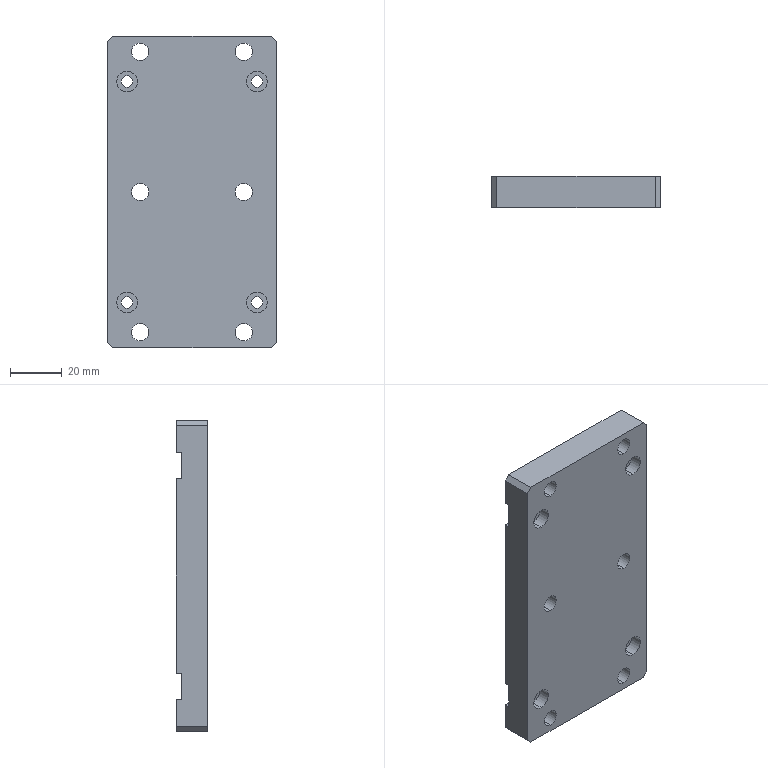Part | SolidWorks | features HoleWzd 2, Chamfer 1, Cut 1, Extrusion 1 | 1 solid | 50 faces | box 65 x 12 x 120 mm | volume 87146 mm3 | cylinder 28 | plane 22 | commonest cylinder face diameters 6.6 x12 4.5 x8 8 x8
STEP:
#1=CARTESIAN_POINT('',(25.,4.6,-38.5));
#2=VERTEX_POINT('',#1);
#3=CARTESIAN_POINT('',(25.,4.6,-46.5));
#4=VERTEX_POINT('',#3);
#5=CARTESIAN_POINT('',(25.,4.6,-42.5));
#6=DIRECTION('',(0.,-1.,0.));
#7=DIRECTION('',(0.,0.,-1.));
#8=AXIS2_PLACEMENT_3D('',#5,#6,#7);
#9=CIRCLE('',#8,4.);
#10=EDGE_CURVE('',#2,#4,#9,.T.);
#11=ORIENTED_EDGE('',*,*,#10,.F.);
#12=CARTESIAN_POINT('',(25.,0.,-38.5));
#13=VERTEX_POINT('',#12);
#14=CARTESIAN_POINT('',(25.,0.,-38.5));
#15=DIRECTION('',(0.,-1.,0.));
#16=VECTOR('',#15,1000.);
#17=LINE('',#14,#16);
#18=EDGE_CURVE('',#2,#13,#17,.T.);
#19=ORIENTED_EDGE('',*,*,#18,.T.);
#20=CARTESIAN_POINT('',(25.,0.,-46.5));
#21=VERTEX_POINT('',#20);
#22=CARTESIAN_POINT('',(25.,0.,-42.5));
#23=DIRECTION('',(0.,-1.,0.));
#24=DIRECTION('',(0.,0.,-1.));
#25=AXIS2_PLACEMENT_3D('',#22,#23,#24);
#26=CIRCLE('',#25,4.);
#27=EDGE_CURVE('',#13,#21,#26,.T.);
#28=ORIENTED_EDGE('',*,*,#27,.T.);
#29=CARTESIAN_POINT('',(25.,0.,-46.5));
#30=DIRECTION('',(0.,-1.,0.));
#31=VECTOR('',#30,1000.);
#32=LINE('',#29,#31);
#33=EDGE_CURVE('',#4,#21,#32,.T.);
#34=ORIENTED_EDGE('',*,*,#33,.F.);
#35=EDGE_LOOP('',(#11,#19,#28,#34));
#36=FACE_OUTER_BOUND('',#35,.T.);
#37=CARTESIAN_POINT('',(25.,0.,-42.5));
#38=DIRECTION('',(0.,-1.,0.));
#39=DIRECTION('',(0.,0.,-1.));
#40=AXIS2_PLACEMENT_3D('',#37,#38,#39);
#41=CYLINDRICAL_SURFACE('',#40,4.);
#42=ADVANCED_FACE('',(#36),#41,.F.);
#43=CARTESIAN_POINT('',(25.,10.,-40.25));
#44=VERTEX_POINT('',#43);
#45=CARTESIAN_POINT('',(25.,10.,-44.75));
#46=VERTEX_POINT('',#45);
#47=CARTESIAN_POINT('',(25.,10.,-42.5));
#48=DIRECTION('',(0.,-1.,0.));
#49=DIRECTION('',(0.,0.,-1.));
#50=AXIS2_PLACEMENT_3D('',#47,#48,#49);
#51=CIRCLE('',#50,2.25);
#52=EDGE_CURVE('',#44,#46,#51,.T.);
#53=ORIENTED_EDGE('',*,*,#52,.F.);
#54=CARTESIAN_POINT('',(25.,4.6,-40.25));
#55=VERTEX_POINT('',#54);
#56=CARTESIAN_POINT('',(25.,0.,-40.25));
#57=DIRECTION('',(0.,-1.,0.));
#58=VECTOR('',#57,1000.);
#59=LINE('',#56,#58);
#60=EDGE_CURVE('',#44,#55,#59,.T.);
#61=ORIENTED_EDGE('',*,*,#60,.T.);
#62=CARTESIAN_POINT('',(25.,4.6,-44.75));
#63=VERTEX_POINT('',#62);
#64=CARTESIAN_POINT('',(25.,4.6,-42.5));
#65=DIRECTION('',(0.,-1.,0.));
#66=DIRECTION('',(0.,0.,-1.));
#67=AXIS2_PLACEMENT_3D('',#64,#65,#66);
#68=CIRCLE('',#67,2.25);
#69=EDGE_CURVE('',#55,#63,#68,.T.);
#70=ORIENTED_EDGE('',*,*,#69,.T.);
#71=CARTESIAN_POINT('',(25.,0.,-44.75));
#72=DIRECTION('',(0.,-1.,0.));
#73=VECTOR('',#72,1000.);
#74=LINE('',#71,#73);
#75=EDGE_CURVE('',#46,#63,#74,.T.);
#76=ORIENTED_EDGE('',*,*,#75,.F.);
#77=EDGE_LOOP('',(#53,#61,#70,#76));
#78=FACE_OUTER_BOUND('',#77,.T.);
#79=CARTESIAN_POINT('',(25.,0.,-42.5));
#80=DIRECTION('',(0.,-1.,0.));
#81=DIRECTION('',(0.,0.,-1.));
#82=AXIS2_PLACEMENT_3D('',#79,#80,#81);
#83=CYLINDRICAL_SURFACE('',#82,2.25);
#84=ADVANCED_FACE('',(#78),#83,.F.);
#85=CARTESIAN_POINT('',(25.,4.6,46.5));
#86=VERTEX_POINT('',#85);
#87=CARTESIAN_POINT('',(25.,4.6,38.5));
#88=VERTEX_POINT('',#87);
#89=CARTESIAN_POINT('',(25.,4.6,42.5));
#90=DIRECTION('',(0.,-1.,0.));
#91=DIRECTION('',(0.,0.,-1.));
#92=AXIS2_PLACEMENT_3D('',#89,#90,#91);
#93=CIRCLE('',#92,4.);
#94=EDGE_CURVE('',#86,#88,#93,.T.);
#95=ORIENTED_EDGE('',*,*,#94,.F.);
#96=CARTESIAN_POINT('',(25.,0.,46.5));
#97=VERTEX_POINT('',#96);
#98=CARTESIAN_POINT('',(25.,0.,46.5));
#99=DIRECTION('',(0.,-1.,0.));
#100=VECTOR('',#99,1000.);
#101=LINE('',#98,#100);
#102=EDGE_CURVE('',#86,#97,#101,.T.);
#103=ORIENTED_EDGE('',*,*,#102,.T.);
#104=CARTESIAN_POINT('',(25.,0.,38.5));
#105=VERTEX_POINT('',#104);
#106=CARTESIAN_POINT('',(25.,0.,42.5));
#107=DIRECTION('',(0.,-1.,0.));
#108=DIRECTION('',(0.,0.,-1.));
#109=AXIS2_PLACEMENT_3D('',#106,#107,#108);
#110=CIRCLE('',#109,4.);
#111=EDGE_CURVE('',#97,#105,#110,.T.);
#112=ORIENTED_EDGE('',*,*,#111,.T.);
#113=CARTESIAN_POINT('',(25.,0.,38.5));
#114=DIRECTION('',(0.,-1.,0.));
#115=VECTOR('',#114,1000.);
#116=LINE('',#113,#115);
#117=EDGE_CURVE('',#88,#105,#116,.T.);
#118=ORIENTED_EDGE('',*,*,#117,.F.);
#119=EDGE_LOOP('',(#95,#103,#112,#118));
#120=FACE_OUTER_BOUND('',#119,.T.);
#121=CARTESIAN_POINT('',(25.,0.,42.5));
#122=DIRECTION('',(0.,-1.,0.));
#123=DIRECTION('',(0.,0.,-1.));
#124=AXIS2_PLACEMENT_3D('',#121,#122,#123);
#125=CYLINDRICAL_SURFACE('',#124,4.);
#126=ADVANCED_FACE('',(#120),#125,.F.);
#127=CARTESIAN_POINT('',(25.,10.,44.75));
#128=VERTEX_POINT('',#127);
#129=CARTESIAN_POINT('',(25.,10.,40.25));
#130=VERTEX_POINT('',#129);
#131=CARTESIAN_POINT('',(25.,10.,42.5));
#132=DIRECTION('',(0.,-1.,0.));
#133=DIRECTION('',(0.,0.,-1.));
#134=AXIS2_PLACEMENT_3D('',#131,#132,#133);
#135=CIRCLE('',#134,2.25);
#136=EDGE_CURVE('',#128,#130,#135,.T.);
#137=ORIENTED_EDGE('',*,*,#136,.F.);
#138=CARTESIAN_POINT('',(25.,4.6,44.75));
#139=VERTEX_POINT('',#138);
#140=CARTESIAN_POINT('',(25.,0.,44.75));
#141=DIRECTION('',(0.,-1.,0.));
#142=VECTOR('',#141,1000.);
#143=LINE('',#140,#142);
#144=EDGE_CURVE('',#128,#139,#143,.T.);
#145=ORIENTED_EDGE('',*,*,#144,.T.);
#146=CARTESIAN_POINT('',(25.,4.6,40.25));
#147=VERTEX_POINT('',#146);
#148=CARTESIAN_POINT('',(25.,4.6,42.5));
#149=DIRECTION('',(0.,-1.,0.));
#150=DIRECTION('',(0.,0.,-1.));
#151=AXIS2_PLACEMENT_3D('',#148,#149,#150);
#152=CIRCLE('',#151,2.25);
#153=EDGE_CURVE('',#139,#147,#152,.T.);
#154=ORIENTED_EDGE('',*,*,#153,.T.);
#155=CARTESIAN_POINT('',(25.,0.,40.25));
#156=DIRECTION('',(0.,-1.,0.));
#157=VECTOR('',#156,1000.);
#158=LINE('',#155,#157);
#159=EDGE_CURVE('',#130,#147,#158,.T.);
#160=ORIENTED_EDGE('',*,*,#159,.F.);
#161=EDGE_LOOP('',(#137,#145,#154,#160));
#162=FACE_OUTER_BOUND('',#161,.T.);
#163=CARTESIAN_POINT('',(25.,0.,42.5));
#164=DIRECTION('',(0.,-1.,0.));
#165=DIRECTION('',(0.,0.,-1.));
#166=AXIS2_PLACEMENT_3D('',#163,#164,#165);
#167=CYLINDRICAL_SURFACE('',#166,2.25);
#168=ADVANCED_FACE('',(#162),#167,.F.);
#169=CARTESIAN_POINT('',(-25.,4.6,46.5));
#170=VERTEX_POINT('',#169);
#171=CARTESIAN_POINT('',(-25.,4.6,38.5));
#172=VERTEX_POINT('',#171);
#173=CARTESIAN_POINT('',(-25.,4.6,42.5));
#174=DIRECTION('',(0.,-1.,0.));
#175=DIRECTION('',(0.,0.,-1.));
#176=AXIS2_PLACEMENT_3D('',#173,#174,#175);
#177=CIRCLE('',#176,4.);
#178=EDGE_CURVE('',#170,#172,#177,.T.);
#179=ORIENTED_EDGE('',*,*,#178,.F.);
#180=CARTESIAN_POINT('',(-25.,0.,46.5));
#181=VERTEX_POINT('',#180);
#182=CARTESIAN_POINT('',(-25.,0.,46.5));
#183=DIRECTION('',(0.,-1.,0.));
#184=VECTOR('',#183,1000.);
#185=LINE('',#182,#184);
#186=EDGE_CURVE('',#170,#181,#185,.T.);
#187=ORIENTED_EDGE('',*,*,#186,.T.);
#188=CARTESIAN_POINT('',(-25.,0.,38.5));
#189=VERTEX_POINT('',#188);
#190=CARTESIAN_POINT('',(-25.,0.,42.5));
#191=DIRECTION('',(0.,-1.,0.));
#192=DIRECTION('',(0.,0.,-1.));
#193=AXIS2_PLACEMENT_3D('',#190,#191,#192);
#194=CIRCLE('',#193,4.);
#195=EDGE_CURVE('',#181,#189,#194,.T.);
#196=ORIENTED_EDGE('',*,*,#195,.T.);
#197=CARTESIAN_POINT('',(-25.,0.,38.5));
#198=DIRECTION('',(0.,-1.,0.));
#199=VECTOR('',#198,1000.);
#200=LINE('',#197,#199);
#201=EDGE_CURVE('',#172,#189,#200,.T.);
#202=ORIENTED_EDGE('',*,*,#201,.F.);
#203=EDGE_LOOP('',(#179,#187,#196,#202));
#204=FACE_OUTER_BOUND('',#203,.T.);
#205=CARTESIAN_POINT('',(-25.,0.,42.5));
#206=DIRECTION('',(0.,-1.,0.));
#207=DIRECTION('',(0.,0.,-1.));
#208=AXIS2_PLACEMENT_3D('',#205,#206,#207);
#209=CYLINDRICAL_SURFACE('',#208,4.);
#210=ADVANCED_FACE('',(#204),#209,.F.);
#211=CARTESIAN_POINT('',(-25.,10.,44.75));
#212=VERTEX_POINT('',#211);
#213=CARTESIAN_POINT('',(-25.,10.,40.25));
#214=VERTEX_POINT('',#213);
#215=CARTESIAN_POINT('',(-25.,10.,42.5));
#216=DIRECTION('',(0.,-1.,0.));
#217=DIRECTION('',(0.,0.,-1.));
#218=AXIS2_PLACEMENT_3D('',#215,#216,#217);
#219=CIRCLE('',#218,2.25);
#220=EDGE_CURVE('',#212,#214,#219,.T.);
#221=ORIENTED_EDGE('',*,*,#220,.F.);
#222=CARTESIAN_POINT('',(-25.,4.6,44.75));
#223=VERTEX_POINT('',#222);
#224=CARTESIAN_POINT('',(-25.,0.,44.75));
#225=DIRECTION('',(0.,-1.,0.));
#226=VECTOR('',#225,1000.);
#227=LINE('',#224,#226);
#228=EDGE_CURVE('',#212,#223,#227,.T.);
#229=ORIENTED_EDGE('',*,*,#228,.T.);
#230=CARTESIAN_POINT('',(-25.,4.6,40.25));
#231=VERTEX_POINT('',#230);
#232=CARTESIAN_POINT('',(-25.,4.6,42.5));
#233=DIRECTION('',(0.,-1.,0.));
#234=DIRECTION('',(0.,0.,-1.));
#235=AXIS2_PLACEMENT_3D('',#232,#233,#234);
#236=CIRCLE('',#235,2.25);
#237=EDGE_CURVE('',#223,#231,#236,.T.);
#238=ORIENTED_EDGE('',*,*,#237,.T.);
#239=CARTESIAN_POINT('',(-25.,0.,40.25));
#240=DIRECTION('',(0.,-1.,0.));
#241=VECTOR('',#240,1000.);
#242=LINE('',#239,#241);
#243=EDGE_CURVE('',#214,#231,#242,.T.);
#244=ORIENTED_EDGE('',*,*,#243,.F.);
#245=EDGE_LOOP('',(#221,#229,#238,#244));
#246=FACE_OUTER_BOUND('',#245,.T.);
#247=CARTESIAN_POINT('',(-25.,0.,42.5));
#248=DIRECTION('',(0.,-1.,0.));
#249=DIRECTION('',(0.,0.,-1.));
#250=AXIS2_PLACEMENT_3D('',#247,#248,#249);
#251=CYLINDRICAL_SURFACE('',#250,2.25);
#252=ADVANCED_FACE('',(#246),#251,.F.);
#253=CARTESIAN_POINT('',(-25.,4.6,-38.5));
#254=VERTEX_POINT('',#253);
#255=CARTESIAN_POINT('',(-25.,4.6,-46.5));
#256=VERTEX_POINT('',#255);
#257=CARTESIAN_POINT('',(-25.,4.6,-42.5));
#258=DIRECTION('',(0.,-1.,0.));
#259=DIRECTION('',(0.,0.,-1.));
#260=AXIS2_PLACEMENT_3D('',#257,#258,#259);
#261=CIRCLE('',#260,4.);
#262=EDGE_CURVE('',#254,#256,#261,.T.);
#263=ORIENTED_EDGE('',*,*,#262,.F.);
#264=CARTESIAN_POINT('',(-25.,0.,-38.5));
#265=VERTEX_POINT('',#264);
#266=CARTESIAN_POINT('',(-25.,0.,-38.5));
#267=DIRECTION('',(0.,-1.,0.));
#268=VECTOR('',#267,1000.);
#269=LINE('',#266,#268);
#270=EDGE_CURVE('',#254,#265,#269,.T.);
#271=ORIENTED_EDGE('',*,*,#270,.T.);
#272=CARTESIAN_POINT('',(-25.,0.,-46.5));
#273=VERTEX_POINT('',#272);
#274=CARTESIAN_POINT('',(-25.,0.,-42.5));
#275=DIRECTION('',(0.,-1.,0.));
#276=DIRECTION('',(0.,0.,-1.));
#277=AXIS2_PLACEMENT_3D('',#274,#275,#276);
#278=CIRCLE('',#277,4.);
#279=EDGE_CURVE('',#265,#273,#278,.T.);
#280=ORIENTED_EDGE('',*,*,#279,.T.);
#281=CARTESIAN_POINT('',(-25.,0.,-46.5));
#282=DIRECTION('',(0.,-1.,0.));
#283=VECTOR('',#282,1000.);
#284=LINE('',#281,#283);
#285=EDGE_CURVE('',#256,#273,#284,.T.);
#286=ORIENTED_EDGE('',*,*,#285,.F.);
#287=EDGE_LOOP('',(#263,#271,#280,#286));
#288=FACE_OUTER_BOUND('',#287,.T.);
#289=CARTESIAN_POINT('',(-25.,0.,-42.5));
#290=DIRECTION('',(0.,-1.,0.));
#291=DIRECTION('',(0.,0.,-1.));
#292=AXIS2_PLACEMENT_3D('',#289,#290,#291);
#293=CYLINDRICAL_SURFACE('',#292,4.);
#294=ADVANCED_FACE('',(#288),#293,.F.);
#295=CARTESIAN_POINT('',(-25.,10.,-40.25));
#296=VERTEX_POINT('',#295);
#297=CARTESIAN_POINT('',(-25.,10.,-44.75));
#298=VERTEX_POINT('',#297);
#299=CARTESIAN_POINT('',(-25.,10.,-42.5));
#300=DIRECTION('',(0.,-1.,0.));
#301=DIRECTION('',(0.,0.,-1.));
#302=AXIS2_PLACEMENT_3D('',#299,#300,#301);
#303=CIRCLE('',#302,2.25);
#304=EDGE_CURVE('',#296,#298,#303,.T.);
#305=ORIENTED_EDGE('',*,*,#304,.F.);
#306=CARTESIAN_POINT('',(-25.,4.6,-40.25));
#307=VERTEX_POINT('',#306);
#308=CARTESIAN_POINT('',(-25.,0.,-40.25));
#309=DIRECTION('',(0.,-1.,0.));
#310=VECTOR('',#309,1000.);
#311=LINE('',#308,#310);
#312=EDGE_CURVE('',#296,#307,#311,.T.);
#313=ORIENTED_EDGE('',*,*,#312,.T.);
#314=CARTESIAN_POINT('',(-25.,4.6,-44.75));
#315=VERTEX_POINT('',#314);
#316=CARTESIAN_POINT('',(-25.,4.6,-42.5));
#317=DIRECTION('',(0.,-1.,0.));
#318=DIRECTION('',(0.,0.,-1.));
#319=AXIS2_PLACEMENT_3D('',#316,#317,#318);
#320=CIRCLE('',#319,2.25);
#321=EDGE_CURVE('',#307,#315,#320,.T.);
#322=ORIENTED_EDGE('',*,*,#321,.T.);
#323=CARTESIAN_POINT('',(-25.,0.,-44.75));
#324=DIRECTION('',(0.,-1.,0.));
#325=VECTOR('',#324,1000.);
#326=LINE('',#323,#325);
#327=EDGE_CURVE('',#298,#315,#326,.T.);
#328=ORIENTED_EDGE('',*,*,#327,.F.);
#329=EDGE_LOOP('',(#305,#313,#322,#328));
#330=FACE_OUTER_BOUND('',#329,.T.);
#331=CARTESIAN_POINT('',(-25.,0.,-42.5));
#332=DIRECTION('',(0.,-1.,0.));
#333=DIRECTION('',(0.,0.,-1.));
#334=AXIS2_PLACEMENT_3D('',#331,#332,#333);
#335=CYLINDRICAL_SURFACE('',#334,2.25);
#336=ADVANCED_FACE('',(#330),#335,.F.);
#337=CARTESIAN_POINT('',(-20.,0.,50.7));
#338=VERTEX_POINT('',#337);
#339=CARTESIAN_POINT('',(-20.,0.,57.3));
#340=VERTEX_POINT('',#339);
#341=CARTESIAN_POINT('',(-20.,0.,54.));
#342=DIRECTION('',(0.,1.,0.));
#343=DIRECTION('',(0.,0.,1.));
#344=AXIS2_PLACEMENT_3D('',#341,#342,#343);
#345=CIRCLE('',#344,3.3);
#346=EDGE_CURVE('',#338,#340,#345,.T.);
#347=ORIENTED_EDGE('',*,*,#346,.F.);
#348=CARTESIAN_POINT('',(-20.,12.,50.7));
#349=VERTEX_POINT('',#348);
#350=CARTESIAN_POINT('',(-20.,12.,50.7));
#351=DIRECTION('',(0.,1.,0.));
#352=VECTOR('',#351,1000.);
#353=LINE('',#350,#352);
#354=EDGE_CURVE('',#338,#349,#353,.T.);
#355=ORIENTED_EDGE('',*,*,#354,.T.);
#356=CARTESIAN_POINT('',(-20.,12.,57.3));
#357=VERTEX_POINT('',#356);
#358=CARTESIAN_POINT('',(-20.,12.,54.));
#359=DIRECTION('',(0.,1.,0.));
#360=DIRECTION('',(0.,0.,1.));
#361=AXIS2_PLACEMENT_3D('',#358,#359,#360);
#362=CIRCLE('',#361,3.3);
#363=EDGE_CURVE('',#349,#357,#362,.T.);
#364=ORIENTED_EDGE('',*,*,#363,.T.);
#365=CARTESIAN_POINT('',(-20.,12.,57.3));
#366=DIRECTION('',(0.,1.,0.));
#367=VECTOR('',#366,1000.);
#368=LINE('',#365,#367);
#369=EDGE_CURVE('',#340,#357,#368,.T.);
#370=ORIENTED_EDGE('',*,*,#369,.F.);
#371=EDGE_LOOP('',(#347,#355,#364,#370));
#372=FACE_OUTER_BOUND('',#371,.T.);
#373=CARTESIAN_POINT('',(-20.,12.,54.));
#374=DIRECTION('',(0.,1.,0.));
#375=DIRECTION('',(0.,0.,1.));
#376=AXIS2_PLACEMENT_3D('',#373,#374,#375);
#377=CYLINDRICAL_SURFACE('',#376,3.3);
#378=ADVANCED_FACE('',(#372),#377,.F.);
#379=CARTESIAN_POINT('',(20.,0.,50.7));
#380=VERTEX_POINT('',#379);
#381=CARTESIAN_POINT('',(20.,0.,57.3));
#382=VERTEX_POINT('',#381);
#383=CARTESIAN_POINT('',(20.,0.,54.));
#384=DIRECTION('',(0.,1.,0.));
#385=DIRECTION('',(0.,0.,1.));
#386=AXIS2_PLACEMENT_3D('',#383,#384,#385);
#387=CIRCLE('',#386,3.3);
#388=EDGE_CURVE('',#380,#382,#387,.T.);
#389=ORIENTED_EDGE('',*,*,#388,.F.);
#390=CARTESIAN_POINT('',(20.,12.,50.7));
#391=VERTEX_POINT('',#390);
#392=CARTESIAN_POINT('',(20.,12.,50.7));
#393=DIRECTION('',(0.,1.,0.));
#394=VECTOR('',#393,1000.);
#395=LINE('',#392,#394);
#396=EDGE_CURVE('',#380,#391,#395,.T.);
#397=ORIENTED_EDGE('',*,*,#396,.T.);
#398=CARTESIAN_POINT('',(20.,12.,57.3));
#399=VERTEX_POINT('',#398);
#400=CARTESIAN_POINT('',(20.,12.,54.));
#401=DIRECTION('',(0.,1.,0.));
#402=DIRECTION('',(0.,0.,1.));
#403=AXIS2_PLACEMENT_3D('',#400,#401,#402);
#404=CIRCLE('',#403,3.3);
#405=EDGE_CURVE('',#391,#399,#404,.T.);
#406=ORIENTED_EDGE('',*,*,#405,.T.);
#407=CARTESIAN_POINT('',(20.,12.,57.3));
#408=DIRECTION('',(0.,1.,0.));
#409=VECTOR('',#408,1000.);
#410=LINE('',#407,#409);
#411=EDGE_CURVE('',#382,#399,#410,.T.);
#412=ORIENTED_EDGE('',*,*,#411,.F.);
#413=EDGE_LOOP('',(#389,#397,#406,#412));
#414=FACE_OUTER_BOUND('',#413,.T.);
#415=CARTESIAN_POINT('',(20.,12.,54.));
#416=DIRECTION('',(0.,1.,0.));
#417=DIRECTION('',(0.,0.,1.));
#418=AXIS2_PLACEMENT_3D('',#415,#416,#417);
#419=CYLINDRICAL_SURFACE('',#418,3.3);
#420=ADVANCED_FACE('',(#414),#419,.F.);
#421=CARTESIAN_POINT('',(-20.,0.,-3.3));
#422=VERTEX_POINT('',#421);
#423=CARTESIAN_POINT('',(-20.,0.,3.3));
#424=VERTEX_POINT('',#423);
#425=CARTESIAN_POINT('',(-20.,0.,0.));
#426=DIRECTION('',(0.,1.,0.));
#427=DIRECTION('',(0.,0.,1.));
#428=AXIS2_PLACEMENT_3D('',#425,#426,#427);
#429=CIRCLE('',#428,3.3);
#430=EDGE_CURVE('',#422,#424,#429,.T.);
#431=ORIENTED_EDGE('',*,*,#430,.F.);
#432=CARTESIAN_POINT('',(-20.,12.,-3.3));
#433=VERTEX_POINT('',#432);
#434=CARTESIAN_POINT('',(-20.,12.,-3.3));
#435=DIRECTION('',(0.,1.,0.));
#436=VECTOR('',#435,1000.);
#437=LINE('',#434,#436);
#438=EDGE_CURVE('',#422,#433,#437,.T.);
#439=ORIENTED_EDGE('',*,*,#438,.T.);
#440=CARTESIAN_POINT('',(-20.,12.,3.3));
#441=VERTEX_POINT('',#440);
#442=CARTESIAN_POINT('',(-20.,12.,0.));
#443=DIRECTION('',(0.,1.,0.));
#444=DIRECTION('',(0.,0.,1.));
#445=AXIS2_PLACEMENT_3D('',#442,#443,#444);
#446=CIRCLE('',#445,3.3);
#447=EDGE_CURVE('',#433,#441,#446,.T.);
#448=ORIENTED_EDGE('',*,*,#447,.T.);
#449=CARTESIAN_POINT('',(-20.,12.,3.3));
#450=DIRECTION('',(0.,1.,0.));
#451=VECTOR('',#450,1000.);
#452=LINE('',#449,#451);
#453=EDGE_CURVE('',#424,#441,#452,.T.);
#454=ORIENTED_EDGE('',*,*,#453,.F.);
#455=EDGE_LOOP('',(#431,#439,#448,#454));
#456=FACE_OUTER_BOUND('',#455,.T.);
#457=CARTESIAN_POINT('',(-20.,12.,0.));
#458=DIRECTION('',(0.,1.,0.));
#459=DIRECTION('',(0.,0.,1.));
#460=AXIS2_PLACEMENT_3D('',#457,#458,#459);
#461=CYLINDRICAL_SURFACE('',#460,3.3);
#462=ADVANCED_FACE('',(#456),#461,.F.);
#463=CARTESIAN_POINT('',(20.,0.,-3.3));
#464=VERTEX_POINT('',#463);
#465=CARTESIAN_POINT('',(20.,0.,3.3));
#466=VERTEX_POINT('',#465);
#467=CARTESIAN_POINT('',(20.,0.,0.));
#468=DIRECTION('',(0.,1.,0.));
#469=DIRECTION('',(0.,0.,1.));
#470=AXIS2_PLACEMENT_3D('',#467,#468,#469);
#471=CIRCLE('',#470,3.3);
#472=EDGE_CURVE('',#464,#466,#471,.T.);
#473=ORIENTED_EDGE('',*,*,#472,.F.);
#474=CARTESIAN_POINT('',(20.,12.,-3.3));
#475=VERTEX_POINT('',#474);
#476=CARTESIAN_POINT('',(20.,12.,-3.3));
#477=DIRECTION('',(0.,1.,0.));
#478=VECTOR('',#477,1000.);
#479=LINE('',#476,#478);
#480=EDGE_CURVE('',#464,#475,#479,.T.);
#481=ORIENTED_EDGE('',*,*,#480,.T.);
#482=CARTESIAN_POINT('',(20.,12.,3.3));
#483=VERTEX_POINT('',#482);
#484=CARTESIAN_POINT('',(20.,12.,0.));
#485=DIRECTION('',(0.,1.,0.));
#486=DIRECTION('',(0.,0.,1.));
#487=AXIS2_PLACEMENT_3D('',#484,#485,#486);
#488=CIRCLE('',#487,3.3);
#489=EDGE_CURVE('',#475,#483,#488,.T.);
#490=ORIENTED_EDGE('',*,*,#489,.T.);
#491=CARTESIAN_POINT('',(20.,12.,3.3));
#492=DIRECTION('',(0.,1.,0.));
#493=VECTOR('',#492,1000.);
#494=LINE('',#491,#493);
#495=EDGE_CURVE('',#466,#483,#494,.T.);
#496=ORIENTED_EDGE('',*,*,#495,.F.);
#497=EDGE_LOOP('',(#473,#481,#490,#496));
#498=FACE_OUTER_BOUND('',#497,.T.);
#499=CARTESIAN_POINT('',(20.,12.,0.));
#500=DIRECTION('',(0.,1.,0.));
#501=DIRECTION('',(0.,0.,1.));
#502=AXIS2_PLACEMENT_3D('',#499,#500,#501);
#503=CYLINDRICAL_SURFACE('',#502,3.3);
#504=ADVANCED_FACE('',(#498),#503,.F.);
#505=CARTESIAN_POINT('',(-20.,0.,-57.3));
#506=VERTEX_POINT('',#505);
#507=CARTESIAN_POINT('',(-20.,0.,-50.7));
#508=VERTEX_POINT('',#507);
#509=CARTESIAN_POINT('',(-20.,0.,-54.));
#510=DIRECTION('',(0.,1.,0.));
#511=DIRECTION('',(0.,0.,1.));
#512=AXIS2_PLACEMENT_3D('',#509,#510,#511);
#513=CIRCLE('',#512,3.3);
#514=EDGE_CURVE('',#506,#508,#513,.T.);
#515=ORIENTED_EDGE('',*,*,#514,.F.);
#516=CARTESIAN_POINT('',(-20.,12.,-57.3));
#517=VERTEX_POINT('',#516);
#518=CARTESIAN_POINT('',(-20.,12.,-57.3));
#519=DIRECTION('',(0.,1.,0.));
#520=VECTOR('',#519,1000.);
#521=LINE('',#518,#520);
#522=EDGE_CURVE('',#506,#517,#521,.T.);
#523=ORIENTED_EDGE('',*,*,#522,.T.);
#524=CARTESIAN_POINT('',(-20.,12.,-50.7));
#525=VERTEX_POINT('',#524);
#526=CARTESIAN_POINT('',(-20.,12.,-54.));
#527=DIRECTION('',(0.,1.,0.));
#528=DIRECTION('',(0.,0.,1.));
#529=AXIS2_PLACEMENT_3D('',#526,#527,#528);
#530=CIRCLE('',#529,3.3);
#531=EDGE_CURVE('',#517,#525,#530,.T.);
#532=ORIENTED_EDGE('',*,*,#531,.T.);
#533=CARTESIAN_POINT('',(-20.,12.,-50.7));
#534=DIRECTION('',(0.,1.,0.));
#535=VECTOR('',#534,1000.);
#536=LINE('',#533,#535);
#537=EDGE_CURVE('',#508,#525,#536,.T.);
#538=ORIENTED_EDGE('',*,*,#537,.F.);
#539=EDGE_LOOP('',(#515,#523,#532,#538));
#540=FACE_OUTER_BOUND('',#539,.T.);
#541=CARTESIAN_POINT('',(-20.,12.,-54.));
#542=DIRECTION('',(0.,1.,0.));
#543=DIRECTION('',(0.,0.,1.));
#544=AXIS2_PLACEMENT_3D('',#541,#542,#543);
#545=CYLINDRICAL_SURFACE('',#544,3.3);
#546=ADVANCED_FACE('',(#540),#545,.F.);
#547=CARTESIAN_POINT('',(20.,0.,-57.3));
#548=VERTEX_POINT('',#547);
#549=CARTESIAN_POINT('',(20.,0.,-50.7));
#550=VERTEX_POINT('',#549);
#551=CARTESIAN_POINT('',(20.,0.,-54.));
#552=DIRECTION('',(0.,1.,0.));
#553=DIRECTION('',(0.,0.,1.));
#554=AXIS2_PLACEMENT_3D('',#551,#552,#553);
#555=CIRCLE('',#554,3.3);
#556=EDGE_CURVE('',#548,#550,#555,.T.);
#557=ORIENTED_EDGE('',*,*,#556,.F.);
#558=CARTESIAN_POINT('',(20.,12.,-57.3));
#559=VERTEX_POINT('',#558);
#560=CARTESIAN_POINT('',(20.,12.,-57.3));
#561=DIRECTION('',(0.,1.,0.));
#562=VECTOR('',#561,1000.);
#563=LINE('',#560,#562);
#564=EDGE_CURVE('',#548,#559,#563,.T.);
#565=ORIENTED_EDGE('',*,*,#564,.T.);
#566=CARTESIAN_POINT('',(20.,12.,-50.7));
#567=VERTEX_POINT('',#566);
#568=CARTESIAN_POINT('',(20.,12.,-54.));
#569=DIRECTION('',(0.,1.,0.));
#570=DIRECTION('',(0.,0.,1.));
#571=AXIS2_PLACEMENT_3D('',#568,#569,#570);
#572=CIRCLE('',#571,3.3);
#573=EDGE_CURVE('',#559,#567,#572,.T.);
#574=ORIENTED_EDGE('',*,*,#573,.T.);
#575=CARTESIAN_POINT('',(20.,12.,-50.7));
#576=DIRECTION('',(0.,1.,0.));
#577=VECTOR('',#576,1000.);
#578=LINE('',#575,#577);
#579=EDGE_CURVE('',#550,#567,#578,.T.);
#580=ORIENTED_EDGE('',*,*,#579,.F.);
#581=EDGE_LOOP('',(#557,#565,#574,#580));
#582=FACE_OUTER_BOUND('',#581,.T.);
#583=CARTESIAN_POINT('',(20.,12.,-54.));
#584=DIRECTION('',(0.,1.,0.));
#585=DIRECTION('',(0.,0.,1.));
#586=AXIS2_PLACEMENT_3D('',#583,#584,#585);
#587=CYLINDRICAL_SURFACE('',#586,3.3);
#588=ADVANCED_FACE('',(#582),#587,.F.);
#589=CARTESIAN_POINT('',(-20.,0.,54.));
#590=DIRECTION('',(0.,1.,0.));
#591=DIRECTION('',(0.,0.,1.));
#592=AXIS2_PLACEMENT_3D('',#589,#590,#591);
#593=CIRCLE('',#592,3.3);
#594=EDGE_CURVE('',#340,#338,#593,.T.);
#595=ORIENTED_EDGE('',*,*,#594,.T.);
#596=ORIENTED_EDGE('',*,*,#346,.T.);
#597=EDGE_LOOP('',(#595,#596));
#598=FACE_BOUND('',#597,.T.);
#599=CARTESIAN_POINT('',(20.,0.,54.));
#600=DIRECTION('',(0.,1.,0.));
#601=DIRECTION('',(0.,0.,1.));
#602=AXIS2_PLACEMENT_3D('',#599,#600,#601);
#603=CIRCLE('',#602,3.3);
#604=EDGE_CURVE('',#382,#380,#603,.T.);
#605=ORIENTED_EDGE('',*,*,#604,.T.);
#606=ORIENTED_EDGE('',*,*,#388,.T.);
#607=EDGE_LOOP('',(#605,#606));
#608=FACE_BOUND('',#607,.T.);
#609=CARTESIAN_POINT('',(-20.,0.,0.));
#610=DIRECTION('',(0.,1.,0.));
#611=DIRECTION('',(0.,0.,1.));
#612=AXIS2_PLACEMENT_3D('',#609,#610,#611);
#613=CIRCLE('',#612,3.3);
#614=EDGE_CURVE('',#424,#422,#613,.T.);
#615=ORIENTED_EDGE('',*,*,#614,.T.);
#616=ORIENTED_EDGE('',*,*,#430,.T.);
#617=EDGE_LOOP('',(#615,#616));
#618=FACE_BOUND('',#617,.T.);
#619=CARTESIAN_POINT('',(20.,0.,0.));
#620=DIRECTION('',(0.,1.,0.));
#621=DIRECTION('',(0.,0.,1.));
#622=AXIS2_PLACEMENT_3D('',#619,#620,#621);
#623=CIRCLE('',#622,3.3);
#624=EDGE_CURVE('',#466,#464,#623,.T.);
#625=ORIENTED_EDGE('',*,*,#624,.T.);
#626=ORIENTED_EDGE('',*,*,#472,.T.);
#627=EDGE_LOOP('',(#625,#626));
#628=FACE_BOUND('',#627,.T.);
#629=CARTESIAN_POINT('',(-20.,0.,-54.));
#630=DIRECTION('',(0.,1.,0.));
#631=DIRECTION('',(0.,0.,1.));
#632=AXIS2_PLACEMENT_3D('',#629,#630,#631);
#633=CIRCLE('',#632,3.3);
#634=EDGE_CURVE('',#508,#506,#633,.T.);
#635=ORIENTED_EDGE('',*,*,#634,.T.);
#636=ORIENTED_EDGE('',*,*,#514,.T.);
#637=EDGE_LOOP('',(#635,#636));
#638=FACE_BOUND('',#637,.T.);
#639=CARTESIAN_POINT('',(20.,0.,-54.));
#640=DIRECTION('',(0.,1.,0.));
#641=DIRECTION('',(0.,0.,1.));
#642=AXIS2_PLACEMENT_3D('',#639,#640,#641);
#643=CIRCLE('',#642,3.3);
#644=EDGE_CURVE('',#550,#548,#643,.T.);
#645=ORIENTED_EDGE('',*,*,#644,.T.);
#646=ORIENTED_EDGE('',*,*,#556,.T.);
#647=EDGE_LOOP('',(#645,#646));
#648=FACE_BOUND('',#647,.T.);
#649=CARTESIAN_POINT('',(-32.5,0.,-58.));
#650=VERTEX_POINT('',#649);
#651=CARTESIAN_POINT('',(-32.5,0.,58.));
#652=VERTEX_POINT('',#651);
#653=CARTESIAN_POINT('',(-32.5,0.,-60.));
#654=DIRECTION('',(0.,0.,1.));
#655=VECTOR('',#654,1000.);
#656=LINE('',#653,#655);
#657=EDGE_CURVE('',#650,#652,#656,.T.);
#658=ORIENTED_EDGE('',*,*,#657,.F.);
#659=CARTESIAN_POINT('',(-30.5,0.,-60.));
#660=VERTEX_POINT('',#659);
#661=CARTESIAN_POINT('',(-32.5,0.,-58.));
#662=DIRECTION('',(0.7071,0.,-0.7071));
#663=VECTOR('',#662,1000.);
#664=LINE('',#661,#663);
#665=EDGE_CURVE('',#650,#660,#664,.T.);
#666=ORIENTED_EDGE('',*,*,#665,.T.);
#667=CARTESIAN_POINT('',(30.5,0.,-60.));
#668=VERTEX_POINT('',#667);
#669=CARTESIAN_POINT('',(-32.5,0.,-60.));
#670=DIRECTION('',(-1.,0.,0.));
#671=VECTOR('',#670,1000.);
#672=LINE('',#669,#671);
#673=EDGE_CURVE('',#668,#660,#672,.T.);
#674=ORIENTED_EDGE('',*,*,#673,.F.);
#675=CARTESIAN_POINT('',(32.5,0.,-58.));
#676=VERTEX_POINT('',#675);
#677=CARTESIAN_POINT('',(30.5,0.,-60.));
#678=DIRECTION('',(0.7071,0.,0.7071));
#679=VECTOR('',#678,1000.);
#680=LINE('',#677,#679);
#681=EDGE_CURVE('',#668,#676,#680,.T.);
#682=ORIENTED_EDGE('',*,*,#681,.T.);
#683=CARTESIAN_POINT('',(32.5,0.,58.));
#684=VERTEX_POINT('',#683);
#685=CARTESIAN_POINT('',(32.5,0.,-60.));
#686=DIRECTION('',(0.,0.,-1.));
#687=VECTOR('',#686,1000.);
#688=LINE('',#685,#687);
#689=EDGE_CURVE('',#684,#676,#688,.T.);
#690=ORIENTED_EDGE('',*,*,#689,.F.);
#691=CARTESIAN_POINT('',(30.5,0.,60.));
#692=VERTEX_POINT('',#691);
#693=CARTESIAN_POINT('',(32.5,0.,58.));
#694=DIRECTION('',(-0.7071,0.,0.7071));
#695=VECTOR('',#694,1000.);
#696=LINE('',#693,#695);
#697=EDGE_CURVE('',#684,#692,#696,.T.);
#698=ORIENTED_EDGE('',*,*,#697,.T.);
#699=CARTESIAN_POINT('',(-30.5,0.,60.));
#700=VERTEX_POINT('',#699);
#701=CARTESIAN_POINT('',(-32.5,0.,60.));
#702=DIRECTION('',(1.,0.,0.));
#703=VECTOR('',#702,1000.);
#704=LINE('',#701,#703);
#705=EDGE_CURVE('',#700,#692,#704,.T.);
#706=ORIENTED_EDGE('',*,*,#705,.F.);
#707=CARTESIAN_POINT('',(-30.5,0.,60.));
#708=DIRECTION('',(-0.7071,0.,-0.7071));
#709=VECTOR('',#708,1000.);
#710=LINE('',#707,#709);
#711=EDGE_CURVE('',#700,#652,#710,.T.);
#712=ORIENTED_EDGE('',*,*,#711,.T.);
#713=EDGE_LOOP('',(#658,#666,#674,#682,#690,#698,#706,#712));
#714=FACE_OUTER_BOUND('',#713,.T.);
#715=CARTESIAN_POINT('',(-25.,0.,-42.5));
#716=DIRECTION('',(0.,-1.,0.));
#717=DIRECTION('',(0.,0.,-1.));
#718=AXIS2_PLACEMENT_3D('',#715,#716,#717);
#719=CIRCLE('',#718,4.);
#720=EDGE_CURVE('',#273,#265,#719,.T.);
#721=ORIENTED_EDGE('',*,*,#720,.F.);
#722=ORIENTED_EDGE('',*,*,#279,.F.);
#723=EDGE_LOOP('',(#721,#722));
#724=FACE_BOUND('',#723,.T.);
#725=CARTESIAN_POINT('',(-25.,0.,42.5));
#726=DIRECTION('',(0.,-1.,0.));
#727=DIRECTION('',(0.,0.,-1.));
#728=AXIS2_PLACEMENT_3D('',#725,#726,#727);
#729=CIRCLE('',#728,4.);
#730=EDGE_CURVE('',#189,#181,#729,.T.);
#731=ORIENTED_EDGE('',*,*,#730,.F.);
#732=ORIENTED_EDGE('',*,*,#195,.F.);
#733=EDGE_LOOP('',(#731,#732));
#734=FACE_BOUND('',#733,.T.);
#735=CARTESIAN_POINT('',(25.,0.,42.5));
#736=DIRECTION('',(0.,-1.,0.));
#737=DIRECTION('',(0.,0.,-1.));
#738=AXIS2_PLACEMENT_3D('',#735,#736,#737);
#739=CIRCLE('',#738,4.);
#740=EDGE_CURVE('',#105,#97,#739,.T.);
#741=ORIENTED_EDGE('',*,*,#740,.F.);
#742=ORIENTED_EDGE('',*,*,#111,.F.);
#743=EDGE_LOOP('',(#741,#742));
#744=FACE_BOUND('',#743,.T.);
#745=CARTESIAN_POINT('',(25.,0.,-42.5));
#746=DIRECTION('',(0.,-1.,0.));
#747=DIRECTION('',(0.,0.,-1.));
#748=AXIS2_PLACEMENT_3D('',#745,#746,#747);
#749=CIRCLE('',#748,4.);
#750=EDGE_CURVE('',#21,#13,#749,.T.);
#751=ORIENTED_EDGE('',*,*,#750,.F.);
#752=ORIENTED_EDGE('',*,*,#27,.F.);
#753=EDGE_LOOP('',(#751,#752));
#754=FACE_BOUND('',#753,.T.);
#755=CARTESIAN_POINT('',(0.,0.,0.));
#756=DIRECTION('',(0.,1.,0.));
#757=DIRECTION('',(0.,0.,1.));
#758=AXIS2_PLACEMENT_3D('',#755,#756,#757);
#759=PLANE('',#758);
#760=ADVANCED_FACE('',(#598,#608,#618,#628,#638,#648,#714,#724,#734,#744,#754),#759,.F.);
#761=CARTESIAN_POINT('',(-32.5,12.,-37.45));
#762=VERTEX_POINT('',#761);
#763=CARTESIAN_POINT('',(32.5,12.,-37.45));
#764=VERTEX_POINT('',#763);
#765=CARTESIAN_POINT('',(32.5,12.,-37.45));
#766=DIRECTION('',(1.,0.,0.));
#767=VECTOR('',#766,1000.);
#768=LINE('',#765,#767);
#769=EDGE_CURVE('',#762,#764,#768,.T.);
#770=ORIENTED_EDGE('',*,*,#769,.F.);
#771=CARTESIAN_POINT('',(-32.5,12.,37.45));
#772=VERTEX_POINT('',#771);
#773=CARTESIAN_POINT('',(-32.5,12.,-60.));
#774=DIRECTION('',(0.,0.,1.));
#775=VECTOR('',#774,1000.);
#776=LINE('',#773,#775);
#777=EDGE_CURVE('',#762,#772,#776,.T.);
#778=ORIENTED_EDGE('',*,*,#777,.T.);
#779=CARTESIAN_POINT('',(32.5,12.,37.45));
#780=VERTEX_POINT('',#779);
#781=CARTESIAN_POINT('',(32.5,12.,37.45));
#782=DIRECTION('',(-1.,0.,0.));
#783=VECTOR('',#782,1000.);
#784=LINE('',#781,#783);
#785=EDGE_CURVE('',#780,#772,#784,.T.);
#786=ORIENTED_EDGE('',*,*,#785,.F.);
#787=CARTESIAN_POINT('',(32.5,12.,-60.));
#788=DIRECTION('',(0.,0.,-1.));
#789=VECTOR('',#788,1000.);
#790=LINE('',#787,#789);
#791=EDGE_CURVE('',#780,#764,#790,.T.);
#792=ORIENTED_EDGE('',*,*,#791,.T.);
#793=EDGE_LOOP('',(#770,#778,#786,#792));
#794=FACE_OUTER_BOUND('',#793,.T.);
#795=CARTESIAN_POINT('',(20.,12.,0.));
#796=DIRECTION('',(0.,1.,0.));
#797=DIRECTION('',(0.,0.,1.));
#798=AXIS2_PLACEMENT_3D('',#795,#796,#797);
#799=CIRCLE('',#798,3.3);
#800=EDGE_CURVE('',#483,#475,#799,.T.);
#801=ORIENTED_EDGE('',*,*,#800,.F.);
#802=ORIENTED_EDGE('',*,*,#489,.F.);
#803=EDGE_LOOP('',(#801,#802));
#804=FACE_BOUND('',#803,.T.);
#805=CARTESIAN_POINT('',(-20.,12.,0.));
#806=DIRECTION('',(0.,1.,0.));
#807=DIRECTION('',(0.,0.,1.));
#808=AXIS2_PLACEMENT_3D('',#805,#806,#807);
#809=CIRCLE('',#808,3.3);
#810=EDGE_CURVE('',#441,#433,#809,.T.);
#811=ORIENTED_EDGE('',*,*,#810,.F.);
#812=ORIENTED_EDGE('',*,*,#447,.F.);
#813=EDGE_LOOP('',(#811,#812));
#814=FACE_BOUND('',#813,.T.);
#815=CARTESIAN_POINT('',(0.,12.,0.));
#816=DIRECTION('',(0.,1.,0.));
#817=DIRECTION('',(0.,0.,1.));
#818=AXIS2_PLACEMENT_3D('',#815,#816,#817);
#819=PLANE('',#818);
#820=ADVANCED_FACE('',(#794,#804,#814),#819,.T.);
#821=CARTESIAN_POINT('',(-30.5,12.,60.));
#822=VERTEX_POINT('',#821);
#823=CARTESIAN_POINT('',(30.5,12.,60.));
#824=VERTEX_POINT('',#823);
#825=CARTESIAN_POINT('',(-32.5,12.,60.));
#826=DIRECTION('',(1.,0.,0.));
#827=VECTOR('',#826,1000.);
#828=LINE('',#825,#827);
#829=EDGE_CURVE('',#822,#824,#828,.T.);
#830=ORIENTED_EDGE('',*,*,#829,.T.);
#831=CARTESIAN_POINT('',(32.5,12.,58.));
#832=VERTEX_POINT('',#831);
#833=CARTESIAN_POINT('',(45.25,12.,45.25));
#834=DIRECTION('',(0.7071,0.,-0.7071));
#835=VECTOR('',#834,1000.);
#836=LINE('',#833,#835);
#837=EDGE_CURVE('',#824,#832,#836,.T.);
#838=ORIENTED_EDGE('',*,*,#837,.T.);
#839=CARTESIAN_POINT('',(32.5,12.,47.55));
#840=VERTEX_POINT('',#839);
#841=CARTESIAN_POINT('',(32.5,12.,-60.));
#842=DIRECTION('',(0.,0.,-1.));
#843=VECTOR('',#842,1000.);
#844=LINE('',#841,#843);
#845=EDGE_CURVE('',#832,#840,#844,.T.);
#846=ORIENTED_EDGE('',*,*,#845,.T.);
#847=CARTESIAN_POINT('',(-32.5,12.,47.55));
#848=VERTEX_POINT('',#847);
#849=CARTESIAN_POINT('',(32.5,12.,47.55));
#850=DIRECTION('',(1.,0.,0.));
#851=VECTOR('',#850,1000.);
#852=LINE('',#849,#851);
#853=EDGE_CURVE('',#848,#840,#852,.T.);
#854=ORIENTED_EDGE('',*,*,#853,.F.);
#855=CARTESIAN_POINT('',(-32.5,12.,58.));
#856=VERTEX_POINT('',#855);
#857=CARTESIAN_POINT('',(-32.5,12.,-60.));
#858=DIRECTION('',(0.,0.,1.));
#859=VECTOR('',#858,1000.);
#860=LINE('',#857,#859);
#861=EDGE_CURVE('',#848,#856,#860,.T.);
#862=ORIENTED_EDGE('',*,*,#861,.T.);
#863=CARTESIAN_POINT('',(-45.25,12.,45.25));
#864=DIRECTION('',(0.7071,0.,0.7071));
#865=VECTOR('',#864,1000.);
#866=LINE('',#863,#865);
#867=EDGE_CURVE('',#856,#822,#866,.T.);
#868=ORIENTED_EDGE('',*,*,#867,.T.);
#869=EDGE_LOOP('',(#830,#838,#846,#854,#862,#868));
#870=FACE_OUTER_BOUND('',#869,.T.);
#871=CARTESIAN_POINT('',(20.,12.,54.));
#872=DIRECTION('',(0.,1.,0.));
#873=DIRECTION('',(0.,0.,1.));
#874=AXIS2_PLACEMENT_3D('',#871,#872,#873);
#875=CIRCLE('',#874,3.3);
#876=EDGE_CURVE('',#399,#391,#875,.T.);
#877=ORIENTED_EDGE('',*,*,#876,.F.);
#878=ORIENTED_EDGE('',*,*,#405,.F.);
#879=EDGE_LOOP('',(#877,#878));
#880=FACE_BOUND('',#879,.T.);
#881=CARTESIAN_POINT('',(-20.,12.,54.));
#882=DIRECTION('',(0.,1.,0.));
#883=DIRECTION('',(0.,0.,1.));
#884=AXIS2_PLACEMENT_3D('',#881,#882,#883);
#885=CIRCLE('',#884,3.3);
#886=EDGE_CURVE('',#357,#349,#885,.T.);
#887=ORIENTED_EDGE('',*,*,#886,.F.);
#888=ORIENTED_EDGE('',*,*,#363,.F.);
#889=EDGE_LOOP('',(#887,#888));
#890=FACE_BOUND('',#889,.T.);
#891=CARTESIAN_POINT('',(0.,12.,0.));
#892=DIRECTION('',(0.,1.,0.));
#893=DIRECTION('',(0.,0.,1.));
#894=AXIS2_PLACEMENT_3D('',#891,#892,#893);
#895=PLANE('',#894);
#896=ADVANCED_FACE('',(#870,#880,#890),#895,.T.);
#897=ORIENTED_EDGE('',*,*,#689,.T.);
#898=CARTESIAN_POINT('',(32.5,12.,-58.));
#899=VERTEX_POINT('',#898);
#900=CARTESIAN_POINT('',(32.5,12.,-58.));
#901=DIRECTION('',(0.,1.,0.));
#902=VECTOR('',#901,1000.);
#903=LINE('',#900,#902);
#904=EDGE_CURVE('',#676,#899,#903,.T.);
#905=ORIENTED_EDGE('',*,*,#904,.T.);
#906=CARTESIAN_POINT('',(32.5,12.,-47.55));
#907=VERTEX_POINT('',#906);
#908=CARTESIAN_POINT('',(32.5,12.,-60.));
#909=DIRECTION('',(0.,0.,-1.));
#910=VECTOR('',#909,1000.);
#911=LINE('',#908,#910);
#912=EDGE_CURVE('',#907,#899,#911,.T.);
#913=ORIENTED_EDGE('',*,*,#912,.F.);
#914=CARTESIAN_POINT('',(32.5,10.,-47.55));
#915=VERTEX_POINT('',#914);
#916=CARTESIAN_POINT('',(32.5,10.,-47.55));
#917=DIRECTION('',(0.,1.,0.));
#918=VECTOR('',#917,1000.);
#919=LINE('',#916,#918);
#920=EDGE_CURVE('',#915,#907,#919,.T.);
#921=ORIENTED_EDGE('',*,*,#920,.F.);
#922=CARTESIAN_POINT('',(32.5,10.,-37.45));
#923=VERTEX_POINT('',#922);
#924=CARTESIAN_POINT('',(32.5,10.,-47.55));
#925=DIRECTION('',(0.,0.,-1.));
#926=VECTOR('',#925,1000.);
#927=LINE('',#924,#926);
#928=EDGE_CURVE('',#923,#915,#927,.T.);
#929=ORIENTED_EDGE('',*,*,#928,.F.);
#930=CARTESIAN_POINT('',(32.5,10.,-37.45));
#931=DIRECTION('',(0.,1.,0.));
#932=VECTOR('',#931,1000.);
#933=LINE('',#930,#932);
#934=EDGE_CURVE('',#923,#764,#933,.T.);
#935=ORIENTED_EDGE('',*,*,#934,.T.);
#936=ORIENTED_EDGE('',*,*,#791,.F.);
#937=CARTESIAN_POINT('',(32.5,10.,37.45));
#938=VERTEX_POINT('',#937);
#939=CARTESIAN_POINT('',(32.5,10.,37.45));
#940=DIRECTION('',(0.,1.,0.));
#941=VECTOR('',#940,1000.);
#942=LINE('',#939,#941);
#943=EDGE_CURVE('',#938,#780,#942,.T.);
#944=ORIENTED_EDGE('',*,*,#943,.F.);
#945=CARTESIAN_POINT('',(32.5,10.,47.55));
#946=VERTEX_POINT('',#945);
#947=CARTESIAN_POINT('',(32.5,10.,47.55));
#948=DIRECTION('',(0.,0.,-1.));
#949=VECTOR('',#948,1000.);
#950=LINE('',#947,#949);
#951=EDGE_CURVE('',#946,#938,#950,.T.);
#952=ORIENTED_EDGE('',*,*,#951,.F.);
#953=CARTESIAN_POINT('',(32.5,10.,47.55));
#954=DIRECTION('',(0.,1.,0.));
#955=VECTOR('',#954,1000.);
#956=LINE('',#953,#955);
#957=EDGE_CURVE('',#946,#840,#956,.T.);
#958=ORIENTED_EDGE('',*,*,#957,.T.);
#959=ORIENTED_EDGE('',*,*,#845,.F.);
#960=CARTESIAN_POINT('',(32.5,12.,58.));
#961=DIRECTION('',(0.,-1.,0.));
#962=VECTOR('',#961,1000.);
#963=LINE('',#960,#962);
#964=EDGE_CURVE('',#832,#684,#963,.T.);
#965=ORIENTED_EDGE('',*,*,#964,.T.);
#966=EDGE_LOOP('',(#897,#905,#913,#921,#929,#935,#936,#944,#952,#958,#959,#965));
#967=FACE_OUTER_BOUND('',#966,.T.);
#968=CARTESIAN_POINT('',(32.5,12.,-60.));
#969=DIRECTION('',(-1.,0.,0.));
#970=DIRECTION('',(0.,0.,1.));
#971=AXIS2_PLACEMENT_3D('',#968,#969,#970);
#972=PLANE('',#971);
#973=ADVANCED_FACE('',(#967),#972,.F.);
#974=ORIENTED_EDGE('',*,*,#673,.T.);
#975=CARTESIAN_POINT('',(-30.5,12.,-60.));
#976=VERTEX_POINT('',#975);
#977=CARTESIAN_POINT('',(-30.5,12.,-60.));
#978=DIRECTION('',(0.,1.,0.));
#979=VECTOR('',#978,1000.);
#980=LINE('',#977,#979);
#981=EDGE_CURVE('',#660,#976,#980,.T.);
#982=ORIENTED_EDGE('',*,*,#981,.T.);
#983=CARTESIAN_POINT('',(30.5,12.,-60.));
#984=VERTEX_POINT('',#983);
#985=CARTESIAN_POINT('',(-32.5,12.,-60.));
#986=DIRECTION('',(-1.,0.,0.));
#987=VECTOR('',#986,1000.);
#988=LINE('',#985,#987);
#989=EDGE_CURVE('',#984,#976,#988,.T.);
#990=ORIENTED_EDGE('',*,*,#989,.F.);
#991=CARTESIAN_POINT('',(30.5,12.,-60.));
#992=DIRECTION('',(0.,-1.,0.));
#993=VECTOR('',#992,1000.);
#994=LINE('',#991,#993);
#995=EDGE_CURVE('',#984,#668,#994,.T.);
#996=ORIENTED_EDGE('',*,*,#995,.T.);
#997=EDGE_LOOP('',(#974,#982,#990,#996));
#998=FACE_OUTER_BOUND('',#997,.T.);
#999=CARTESIAN_POINT('',(-32.5,12.,-60.));
#1000=DIRECTION('',(0.,0.,1.));
#1001=DIRECTION('',(1.,0.,0.));
#1002=AXIS2_PLACEMENT_3D('',#999,#1000,#1001);
#1003=PLANE('',#1002);
#1004=ADVANCED_FACE('',(#998),#1003,.F.);
#1005=CARTESIAN_POINT('',(-32.5,12.,-58.));
#1006=VERTEX_POINT('',#1005);
#1007=CARTESIAN_POINT('',(-32.5,12.,-47.55));
#1008=VERTEX_POINT('',#1007);
#1009=CARTESIAN_POINT('',(-32.5,12.,-60.));
#1010=DIRECTION('',(0.,0.,1.));
#1011=VECTOR('',#1010,1000.);
#1012=LINE('',#1009,#1011);
#1013=EDGE_CURVE('',#1006,#1008,#1012,.T.);
#1014=ORIENTED_EDGE('',*,*,#1013,.F.);
#1015=CARTESIAN_POINT('',(-32.5,12.,-58.));
#1016=DIRECTION('',(0.,-1.,0.));
#1017=VECTOR('',#1016,1000.);
#1018=LINE('',#1015,#1017);
#1019=EDGE_CURVE('',#1006,#650,#1018,.T.);
#1020=ORIENTED_EDGE('',*,*,#1019,.T.);
#1021=ORIENTED_EDGE('',*,*,#657,.T.);
#1022=CARTESIAN_POINT('',(-32.5,12.,58.));
#1023=DIRECTION('',(0.,1.,0.));
#1024=VECTOR('',#1023,1000.);
#1025=LINE('',#1022,#1024);
#1026=EDGE_CURVE('',#652,#856,#1025,.T.);
#1027=ORIENTED_EDGE('',*,*,#1026,.T.);
#1028=ORIENTED_EDGE('',*,*,#861,.F.);
#1029=CARTESIAN_POINT('',(-32.5,10.,47.55));
#1030=VERTEX_POINT('',#1029);
#1031=CARTESIAN_POINT('',(-32.5,10.,47.55));
#1032=DIRECTION('',(0.,1.,0.));
#1033=VECTOR('',#1032,1000.);
#1034=LINE('',#1031,#1033);
#1035=EDGE_CURVE('',#1030,#848,#1034,.T.);
#1036=ORIENTED_EDGE('',*,*,#1035,.F.);
#1037=CARTESIAN_POINT('',(-32.5,10.,37.45));
#1038=VERTEX_POINT('',#1037);
#1039=CARTESIAN_POINT('',(-32.5,10.,47.55));
#1040=DIRECTION('',(0.,0.,1.));
#1041=VECTOR('',#1040,1000.);
#1042=LINE('',#1039,#1041);
#1043=EDGE_CURVE('',#1038,#1030,#1042,.T.);
#1044=ORIENTED_EDGE('',*,*,#1043,.F.);
#1045=CARTESIAN_POINT('',(-32.5,10.,37.45));
#1046=DIRECTION('',(0.,1.,0.));
#1047=VECTOR('',#1046,1000.);
#1048=LINE('',#1045,#1047);
#1049=EDGE_CURVE('',#1038,#772,#1048,.T.);
#1050=ORIENTED_EDGE('',*,*,#1049,.T.);
#1051=ORIENTED_EDGE('',*,*,#777,.F.);
#1052=CARTESIAN_POINT('',(-32.5,10.,-37.45));
#1053=VERTEX_POINT('',#1052);
#1054=CARTESIAN_POINT('',(-32.5,10.,-37.45));
#1055=DIRECTION('',(0.,1.,0.));
#1056=VECTOR('',#1055,1000.);
#1057=LINE('',#1054,#1056);
#1058=EDGE_CURVE('',#1053,#762,#1057,.T.);
#1059=ORIENTED_EDGE('',*,*,#1058,.F.);
#1060=CARTESIAN_POINT('',(-32.5,10.,-47.55));
#1061=VERTEX_POINT('',#1060);
#1062=CARTESIAN_POINT('',(-32.5,10.,-47.55));
#1063=DIRECTION('',(0.,0.,1.));
#1064=VECTOR('',#1063,1000.);
#1065=LINE('',#1062,#1064);
#1066=EDGE_CURVE('',#1061,#1053,#1065,.T.);
#1067=ORIENTED_EDGE('',*,*,#1066,.F.);
#1068=CARTESIAN_POINT('',(-32.5,10.,-47.55));
#1069=DIRECTION('',(0.,1.,0.));
#1070=VECTOR('',#1069,1000.);
#1071=LINE('',#1068,#1070);
#1072=EDGE_CURVE('',#1061,#1008,#1071,.T.);
#1073=ORIENTED_EDGE('',*,*,#1072,.T.);
#1074=EDGE_LOOP('',(#1014,#1020,#1021,#1027,#1028,#1036,#1044,#1050,#1051,#1059,#1067,#1073));
#1075=FACE_OUTER_BOUND('',#1074,.T.);
#1076=CARTESIAN_POINT('',(-32.5,12.,-60.));
#1077=DIRECTION('',(1.,0.,0.));
#1078=DIRECTION('',(0.,0.,-1.));
#1079=AXIS2_PLACEMENT_3D('',#1076,#1077,#1078);
#1080=PLANE('',#1079);
#1081=ADVANCED_FACE('',(#1075),#1080,.F.);
#1082=ORIENTED_EDGE('',*,*,#705,.T.);
#1083=CARTESIAN_POINT('',(30.5,12.,60.));
#1084=DIRECTION('',(0.,1.,0.));
#1085=VECTOR('',#1084,1000.);
#1086=LINE('',#1083,#1085);
#1087=EDGE_CURVE('',#692,#824,#1086,.T.);
#1088=ORIENTED_EDGE('',*,*,#1087,.T.);
#1089=ORIENTED_EDGE('',*,*,#829,.F.);
#1090=CARTESIAN_POINT('',(-30.5,12.,60.));
#1091=DIRECTION('',(0.,-1.,0.));
#1092=VECTOR('',#1091,1000.);
#1093=LINE('',#1090,#1092);
#1094=EDGE_CURVE('',#822,#700,#1093,.T.);
#1095=ORIENTED_EDGE('',*,*,#1094,.T.);
#1096=EDGE_LOOP('',(#1082,#1088,#1089,#1095));
#1097=FACE_OUTER_BOUND('',#1096,.T.);
#1098=CARTESIAN_POINT('',(-32.5,12.,60.));
#1099=DIRECTION('',(0.,0.,-1.));
#1100=DIRECTION('',(-1.,0.,0.));
#1101=AXIS2_PLACEMENT_3D('',#1098,#1099,#1100);
#1102=PLANE('',#1101);
#1103=ADVANCED_FACE('',(#1097),#1102,.F.);
#1104=ORIENTED_EDGE('',*,*,#989,.T.);
#1105=CARTESIAN_POINT('',(-45.25,12.,-45.25));
#1106=DIRECTION('',(-0.7071,0.,0.7071));
#1107=VECTOR('',#1106,1000.);
#1108=LINE('',#1105,#1107);
#1109=EDGE_CURVE('',#976,#1006,#1108,.T.);
#1110=ORIENTED_EDGE('',*,*,#1109,.T.);
#1111=ORIENTED_EDGE('',*,*,#1013,.T.);
#1112=CARTESIAN_POINT('',(32.5,12.,-47.55));
#1113=DIRECTION('',(-1.,0.,0.));
#1114=VECTOR('',#1113,1000.);
#1115=LINE('',#1112,#1114);
#1116=EDGE_CURVE('',#907,#1008,#1115,.T.);
#1117=ORIENTED_EDGE('',*,*,#1116,.F.);
#1118=ORIENTED_EDGE('',*,*,#912,.T.);
#1119=CARTESIAN_POINT('',(45.25,12.,-45.25));
#1120=DIRECTION('',(-0.7071,0.,-0.7071));
#1121=VECTOR('',#1120,1000.);
#1122=LINE('',#1119,#1121);
#1123=EDGE_CURVE('',#899,#984,#1122,.T.);
#1124=ORIENTED_EDGE('',*,*,#1123,.T.);
#1125=EDGE_LOOP('',(#1104,#1110,#1111,#1117,#1118,#1124));
#1126=FACE_OUTER_BOUND('',#1125,.T.);
#1127=CARTESIAN_POINT('',(-20.,12.,-54.));
#1128=DIRECTION('',(0.,1.,0.));
#1129=DIRECTION('',(0.,0.,1.));
#1130=AXIS2_PLACEMENT_3D('',#1127,#1128,#1129);
#1131=CIRCLE('',#1130,3.3);
#1132=EDGE_CURVE('',#525,#517,#1131,.T.);
#1133=ORIENTED_EDGE('',*,*,#1132,.F.);
#1134=ORIENTED_EDGE('',*,*,#531,.F.);
#1135=EDGE_LOOP('',(#1133,#1134));
#1136=FACE_BOUND('',#1135,.T.);
#1137=CARTESIAN_POINT('',(20.,12.,-54.));
#1138=DIRECTION('',(0.,1.,0.));
#1139=DIRECTION('',(0.,0.,1.));
#1140=AXIS2_PLACEMENT_3D('',#1137,#1138,#1139);
#1141=CIRCLE('',#1140,3.3);
#1142=EDGE_CURVE('',#567,#559,#1141,.T.);
#1143=ORIENTED_EDGE('',*,*,#1142,.F.);
#1144=ORIENTED_EDGE('',*,*,#573,.F.);
#1145=EDGE_LOOP('',(#1143,#1144));
#1146=FACE_BOUND('',#1145,.T.);
#1147=CARTESIAN_POINT('',(0.,12.,0.));
#1148=DIRECTION('',(0.,1.,0.));
#1149=DIRECTION('',(0.,0.,1.));
#1150=AXIS2_PLACEMENT_3D('',#1147,#1148,#1149);
#1151=PLANE('',#1150);
#1152=ADVANCED_FACE('',(#1126,#1136,#1146),#1151,.T.);
#1153=ORIENTED_EDGE('',*,*,#564,.F.);
#1154=ORIENTED_EDGE('',*,*,#644,.F.);
#1155=ORIENTED_EDGE('',*,*,#579,.T.);
#1156=ORIENTED_EDGE('',*,*,#1142,.T.);
#1157=EDGE_LOOP('',(#1153,#1154,#1155,#1156));
#1158=FACE_OUTER_BOUND('',#1157,.T.);
#1159=CARTESIAN_POINT('',(20.,12.,-54.));
#1160=DIRECTION('',(0.,1.,0.));
#1161=DIRECTION('',(0.,0.,1.));
#1162=AXIS2_PLACEMENT_3D('',#1159,#1160,#1161);
#1163=CYLINDRICAL_SURFACE('',#1162,3.3);
#1164=ADVANCED_FACE('',(#1158),#1163,.F.);
#1165=ORIENTED_EDGE('',*,*,#522,.F.);
#1166=ORIENTED_EDGE('',*,*,#634,.F.);
#1167=ORIENTED_EDGE('',*,*,#537,.T.);
#1168=ORIENTED_EDGE('',*,*,#1132,.T.);
#1169=EDGE_LOOP('',(#1165,#1166,#1167,#1168));
#1170=FACE_OUTER_BOUND('',#1169,.T.);
#1171=CARTESIAN_POINT('',(-20.,12.,-54.));
#1172=DIRECTION('',(0.,1.,0.));
#1173=DIRECTION('',(0.,0.,1.));
#1174=AXIS2_PLACEMENT_3D('',#1171,#1172,#1173);
#1175=CYLINDRICAL_SURFACE('',#1174,3.3);
#1176=ADVANCED_FACE('',(#1170),#1175,.F.);
#1177=ORIENTED_EDGE('',*,*,#480,.F.);
#1178=ORIENTED_EDGE('',*,*,#624,.F.);
#1179=ORIENTED_EDGE('',*,*,#495,.T.);
#1180=ORIENTED_EDGE('',*,*,#800,.T.);
#1181=EDGE_LOOP('',(#1177,#1178,#1179,#1180));
#1182=FACE_OUTER_BOUND('',#1181,.T.);
#1183=CARTESIAN_POINT('',(20.,12.,0.));
#1184=DIRECTION('',(0.,1.,0.));
#1185=DIRECTION('',(0.,0.,1.));
#1186=AXIS2_PLACEMENT_3D('',#1183,#1184,#1185);
#1187=CYLINDRICAL_SURFACE('',#1186,3.3);
#1188=ADVANCED_FACE('',(#1182),#1187,.F.);
#1189=ORIENTED_EDGE('',*,*,#438,.F.);
#1190=ORIENTED_EDGE('',*,*,#614,.F.);
#1191=ORIENTED_EDGE('',*,*,#453,.T.);
#1192=ORIENTED_EDGE('',*,*,#810,.T.);
#1193=EDGE_LOOP('',(#1189,#1190,#1191,#1192));
#1194=FACE_OUTER_BOUND('',#1193,.T.);
#1195=CARTESIAN_POINT('',(-20.,12.,0.));
#1196=DIRECTION('',(0.,1.,0.));
#1197=DIRECTION('',(0.,0.,1.));
#1198=AXIS2_PLACEMENT_3D('',#1195,#1196,#1197);
#1199=CYLINDRICAL_SURFACE('',#1198,3.3);
#1200=ADVANCED_FACE('',(#1194),#1199,.F.);
#1201=ORIENTED_EDGE('',*,*,#396,.F.);
#1202=ORIENTED_EDGE('',*,*,#604,.F.);
#1203=ORIENTED_EDGE('',*,*,#411,.T.);
#1204=ORIENTED_EDGE('',*,*,#876,.T.);
#1205=EDGE_LOOP('',(#1201,#1202,#1203,#1204));
#1206=FACE_OUTER_BOUND('',#1205,.T.);
#1207=CARTESIAN_POINT('',(20.,12.,54.));
#1208=DIRECTION('',(0.,1.,0.));
#1209=DIRECTION('',(0.,0.,1.));
#1210=AXIS2_PLACEMENT_3D('',#1207,#1208,#1209);
#1211=CYLINDRICAL_SURFACE('',#1210,3.3);
#1212=ADVANCED_FACE('',(#1206),#1211,.F.);
#1213=ORIENTED_EDGE('',*,*,#354,.F.);
#1214=ORIENTED_EDGE('',*,*,#594,.F.);
#1215=ORIENTED_EDGE('',*,*,#369,.T.);
#1216=ORIENTED_EDGE('',*,*,#886,.T.);
#1217=EDGE_LOOP('',(#1213,#1214,#1215,#1216));
#1218=FACE_OUTER_BOUND('',#1217,.T.);
#1219=CARTESIAN_POINT('',(-20.,12.,54.));
#1220=DIRECTION('',(0.,1.,0.));
#1221=DIRECTION('',(0.,0.,1.));
#1222=AXIS2_PLACEMENT_3D('',#1219,#1220,#1221);
#1223=CYLINDRICAL_SURFACE('',#1222,3.3);
#1224=ADVANCED_FACE('',(#1218),#1223,.F.);
#1225=ORIENTED_EDGE('',*,*,#853,.T.);
#1226=ORIENTED_EDGE('',*,*,#957,.F.);
#1227=CARTESIAN_POINT('',(32.5,10.,47.55));
#1228=DIRECTION('',(1.,0.,0.));
#1229=VECTOR('',#1228,1000.);
#1230=LINE('',#1227,#1229);
#1231=EDGE_CURVE('',#1030,#946,#1230,.T.);
#1232=ORIENTED_EDGE('',*,*,#1231,.F.);
#1233=ORIENTED_EDGE('',*,*,#1035,.T.);
#1234=EDGE_LOOP('',(#1225,#1226,#1232,#1233));
#1235=FACE_OUTER_BOUND('',#1234,.T.);
#1236=CARTESIAN_POINT('',(32.5,10.,47.55));
#1237=DIRECTION('',(0.,0.,1.));
#1238=DIRECTION('',(1.,0.,0.));
#1239=AXIS2_PLACEMENT_3D('',#1236,#1237,#1238);
#1240=PLANE('',#1239);
#1241=ADVANCED_FACE('',(#1235),#1240,.F.);
#1242=ORIENTED_EDGE('',*,*,#785,.T.);
#1243=ORIENTED_EDGE('',*,*,#1049,.F.);
#1244=CARTESIAN_POINT('',(32.5,10.,37.45));
#1245=DIRECTION('',(-1.,0.,0.));
#1246=VECTOR('',#1245,1000.);
#1247=LINE('',#1244,#1246);
#1248=EDGE_CURVE('',#938,#1038,#1247,.T.);
#1249=ORIENTED_EDGE('',*,*,#1248,.F.);
#1250=ORIENTED_EDGE('',*,*,#943,.T.);
#1251=EDGE_LOOP('',(#1242,#1243,#1249,#1250));
#1252=FACE_OUTER_BOUND('',#1251,.T.);
#1253=CARTESIAN_POINT('',(32.5,10.,37.45));
#1254=DIRECTION('',(0.,0.,-1.));
#1255=DIRECTION('',(-1.,0.,0.));
#1256=AXIS2_PLACEMENT_3D('',#1253,#1254,#1255);
#1257=PLANE('',#1256);
#1258=ADVANCED_FACE('',(#1252),#1257,.F.);
#1259=CARTESIAN_POINT('',(25.,10.,42.5));
#1260=DIRECTION('',(0.,-1.,0.));
#1261=DIRECTION('',(0.,0.,-1.));
#1262=AXIS2_PLACEMENT_3D('',#1259,#1260,#1261);
#1263=CIRCLE('',#1262,2.25);
#1264=EDGE_CURVE('',#130,#128,#1263,.T.);
#1265=ORIENTED_EDGE('',*,*,#1264,.T.);
#1266=ORIENTED_EDGE('',*,*,#136,.T.);
#1267=EDGE_LOOP('',(#1265,#1266));
#1268=FACE_BOUND('',#1267,.T.);
#1269=CARTESIAN_POINT('',(-25.,10.,42.5));
#1270=DIRECTION('',(0.,-1.,0.));
#1271=DIRECTION('',(0.,0.,-1.));
#1272=AXIS2_PLACEMENT_3D('',#1269,#1270,#1271);
#1273=CIRCLE('',#1272,2.25);
#1274=EDGE_CURVE('',#214,#212,#1273,.T.);
#1275=ORIENTED_EDGE('',*,*,#1274,.T.);
#1276=ORIENTED_EDGE('',*,*,#220,.T.);
#1277=EDGE_LOOP('',(#1275,#1276));
#1278=FACE_BOUND('',#1277,.T.);
#1279=ORIENTED_EDGE('',*,*,#1231,.T.);
#1280=ORIENTED_EDGE('',*,*,#951,.T.);
#1281=ORIENTED_EDGE('',*,*,#1248,.T.);
#1282=ORIENTED_EDGE('',*,*,#1043,.T.);
#1283=EDGE_LOOP('',(#1279,#1280,#1281,#1282));
#1284=FACE_OUTER_BOUND('',#1283,.T.);
#1285=CARTESIAN_POINT('',(0.,10.,0.));
#1286=DIRECTION('',(0.,-1.,0.));
#1287=DIRECTION('',(0.,0.,-1.));
#1288=AXIS2_PLACEMENT_3D('',#1285,#1286,#1287);
#1289=PLANE('',#1288);
#1290=ADVANCED_FACE('',(#1268,#1278,#1284),#1289,.F.);
#1291=ORIENTED_EDGE('',*,*,#769,.T.);
#1292=ORIENTED_EDGE('',*,*,#934,.F.);
#1293=CARTESIAN_POINT('',(32.5,10.,-37.45));
#1294=DIRECTION('',(1.,0.,0.));
#1295=VECTOR('',#1294,1000.);
#1296=LINE('',#1293,#1295);
#1297=EDGE_CURVE('',#1053,#923,#1296,.T.);
#1298=ORIENTED_EDGE('',*,*,#1297,.F.);
#1299=ORIENTED_EDGE('',*,*,#1058,.T.);
#1300=EDGE_LOOP('',(#1291,#1292,#1298,#1299));
#1301=FACE_OUTER_BOUND('',#1300,.T.);
#1302=CARTESIAN_POINT('',(32.5,10.,-37.45));
#1303=DIRECTION('',(0.,0.,1.));
#1304=DIRECTION('',(1.,0.,0.));
#1305=AXIS2_PLACEMENT_3D('',#1302,#1303,#1304);
#1306=PLANE('',#1305);
#1307=ADVANCED_FACE('',(#1301),#1306,.F.);
#1308=ORIENTED_EDGE('',*,*,#1116,.T.);
#1309=ORIENTED_EDGE('',*,*,#1072,.F.);
#1310=CARTESIAN_POINT('',(32.5,10.,-47.55));
#1311=DIRECTION('',(-1.,0.,0.));
#1312=VECTOR('',#1311,1000.);
#1313=LINE('',#1310,#1312);
#1314=EDGE_CURVE('',#915,#1061,#1313,.T.);
#1315=ORIENTED_EDGE('',*,*,#1314,.F.);
#1316=ORIENTED_EDGE('',*,*,#920,.T.);
#1317=EDGE_LOOP('',(#1308,#1309,#1315,#1316));
#1318=FACE_OUTER_BOUND('',#1317,.T.);
#1319=CARTESIAN_POINT('',(32.5,10.,-47.55));
#1320=DIRECTION('',(0.,0.,-1.));
#1321=DIRECTION('',(-1.,0.,0.));
#1322=AXIS2_PLACEMENT_3D('',#1319,#1320,#1321);
#1323=PLANE('',#1322);
#1324=ADVANCED_FACE('',(#1318),#1323,.F.);
#1325=CARTESIAN_POINT('',(25.,10.,-42.5));
#1326=DIRECTION('',(0.,-1.,0.));
#1327=DIRECTION('',(0.,0.,-1.));
#1328=AXIS2_PLACEMENT_3D('',#1325,#1326,#1327);
#1329=CIRCLE('',#1328,2.25);
#1330=EDGE_CURVE('',#46,#44,#1329,.T.);
#1331=ORIENTED_EDGE('',*,*,#1330,.T.);
#1332=ORIENTED_EDGE('',*,*,#52,.T.);
#1333=EDGE_LOOP('',(#1331,#1332));
#1334=FACE_BOUND('',#1333,.T.);
#1335=CARTESIAN_POINT('',(-25.,10.,-42.5));
#1336=DIRECTION('',(0.,-1.,0.));
#1337=DIRECTION('',(0.,0.,-1.));
#1338=AXIS2_PLACEMENT_3D('',#1335,#1336,#1337);
#1339=CIRCLE('',#1338,2.25);
#1340=EDGE_CURVE('',#298,#296,#1339,.T.);
#1341=ORIENTED_EDGE('',*,*,#1340,.T.);
#1342=ORIENTED_EDGE('',*,*,#304,.T.);
#1343=EDGE_LOOP('',(#1341,#1342));
#1344=FACE_BOUND('',#1343,.T.);
#1345=ORIENTED_EDGE('',*,*,#928,.T.);
#1346=ORIENTED_EDGE('',*,*,#1314,.T.);
#1347=ORIENTED_EDGE('',*,*,#1066,.T.);
#1348=ORIENTED_EDGE('',*,*,#1297,.T.);
#1349=EDGE_LOOP('',(#1345,#1346,#1347,#1348));
#1350=FACE_OUTER_BOUND('',#1349,.T.);
#1351=CARTESIAN_POINT('',(0.,10.,0.));
#1352=DIRECTION('',(0.,-1.,0.));
#1353=DIRECTION('',(0.,0.,-1.));
#1354=AXIS2_PLACEMENT_3D('',#1351,#1352,#1353);
#1355=PLANE('',#1354);
#1356=ADVANCED_FACE('',(#1334,#1344,#1350),#1355,.F.);
#1357=ORIENTED_EDGE('',*,*,#1109,.F.);
#1358=ORIENTED_EDGE('',*,*,#981,.F.);
#1359=ORIENTED_EDGE('',*,*,#665,.F.);
#1360=ORIENTED_EDGE('',*,*,#1019,.F.);
#1361=EDGE_LOOP('',(#1357,#1358,#1359,#1360));
#1362=FACE_OUTER_BOUND('',#1361,.T.);
#1363=CARTESIAN_POINT('',(-32.5,12.,-58.));
#1364=DIRECTION('',(0.7071,0.,0.7071));
#1365=DIRECTION('',(0.,-1.,0.));
#1366=AXIS2_PLACEMENT_3D('',#1363,#1364,#1365);
#1367=PLANE('',#1366);
#1368=ADVANCED_FACE('',(#1362),#1367,.F.);
#1369=ORIENTED_EDGE('',*,*,#1123,.F.);
#1370=ORIENTED_EDGE('',*,*,#904,.F.);
#1371=ORIENTED_EDGE('',*,*,#681,.F.);
#1372=ORIENTED_EDGE('',*,*,#995,.F.);
#1373=EDGE_LOOP('',(#1369,#1370,#1371,#1372));
#1374=FACE_OUTER_BOUND('',#1373,.T.);
#1375=CARTESIAN_POINT('',(30.5,12.,-60.));
#1376=DIRECTION('',(-0.7071,0.,0.7071));
#1377=DIRECTION('',(0.,-1.,0.));
#1378=AXIS2_PLACEMENT_3D('',#1375,#1376,#1377);
#1379=PLANE('',#1378);
#1380=ADVANCED_FACE('',(#1374),#1379,.F.);
#1381=ORIENTED_EDGE('',*,*,#837,.F.);
#1382=ORIENTED_EDGE('',*,*,#1087,.F.);
#1383=ORIENTED_EDGE('',*,*,#697,.F.);
#1384=ORIENTED_EDGE('',*,*,#964,.F.);
#1385=EDGE_LOOP('',(#1381,#1382,#1383,#1384));
#1386=FACE_OUTER_BOUND('',#1385,.T.);
#1387=CARTESIAN_POINT('',(32.5,12.,58.));
#1388=DIRECTION('',(-0.7071,0.,-0.7071));
#1389=DIRECTION('',(0.,-1.,0.));
#1390=AXIS2_PLACEMENT_3D('',#1387,#1388,#1389);
#1391=PLANE('',#1390);
#1392=ADVANCED_FACE('',(#1386),#1391,.F.);
#1393=ORIENTED_EDGE('',*,*,#867,.F.);
#1394=ORIENTED_EDGE('',*,*,#1026,.F.);
#1395=ORIENTED_EDGE('',*,*,#711,.F.);
#1396=ORIENTED_EDGE('',*,*,#1094,.F.);
#1397=EDGE_LOOP('',(#1393,#1394,#1395,#1396));
#1398=FACE_OUTER_BOUND('',#1397,.T.);
#1399=CARTESIAN_POINT('',(-30.5,12.,60.));
#1400=DIRECTION('',(0.7071,0.,-0.7071));
#1401=DIRECTION('',(0.,-1.,0.));
#1402=AXIS2_PLACEMENT_3D('',#1399,#1400,#1401);
#1403=PLANE('',#1402);
#1404=ADVANCED_FACE('',(#1398),#1403,.F.);
#1405=ORIENTED_EDGE('',*,*,#312,.F.);
#1406=ORIENTED_EDGE('',*,*,#1340,.F.);
#1407=ORIENTED_EDGE('',*,*,#327,.T.);
#1408=CARTESIAN_POINT('',(-25.,4.6,-42.5));
#1409=DIRECTION('',(0.,-1.,0.));
#1410=DIRECTION('',(0.,0.,-1.));
#1411=AXIS2_PLACEMENT_3D('',#1408,#1409,#1410);
#1412=CIRCLE('',#1411,2.25);
#1413=EDGE_CURVE('',#315,#307,#1412,.T.);
#1414=ORIENTED_EDGE('',*,*,#1413,.T.);
#1415=EDGE_LOOP('',(#1405,#1406,#1407,#1414));
#1416=FACE_OUTER_BOUND('',#1415,.T.);
#1417=CARTESIAN_POINT('',(-25.,0.,-42.5));
#1418=DIRECTION('',(0.,-1.,0.));
#1419=DIRECTION('',(0.,0.,-1.));
#1420=AXIS2_PLACEMENT_3D('',#1417,#1418,#1419);
#1421=CYLINDRICAL_SURFACE('',#1420,2.25);
#1422=ADVANCED_FACE('',(#1416),#1421,.F.);
#1423=ORIENTED_EDGE('',*,*,#1413,.F.);
#1424=ORIENTED_EDGE('',*,*,#321,.F.);
#1425=EDGE_LOOP('',(#1423,#1424));
#1426=FACE_BOUND('',#1425,.T.);
#1427=CARTESIAN_POINT('',(-25.,4.6,-42.5));
#1428=DIRECTION('',(0.,-1.,0.));
#1429=DIRECTION('',(0.,0.,-1.));
#1430=AXIS2_PLACEMENT_3D('',#1427,#1428,#1429);
#1431=CIRCLE('',#1430,4.);
#1432=EDGE_CURVE('',#256,#254,#1431,.T.);
#1433=ORIENTED_EDGE('',*,*,#1432,.T.);
#1434=ORIENTED_EDGE('',*,*,#262,.T.);
#1435=EDGE_LOOP('',(#1433,#1434));
#1436=FACE_OUTER_BOUND('',#1435,.T.);
#1437=CARTESIAN_POINT('',(-22.75,4.6,-42.5));
#1438=DIRECTION('',(0.,1.,0.));
#1439=DIRECTION('',(0.,0.,1.));
#1440=AXIS2_PLACEMENT_3D('',#1437,#1438,#1439);
#1441=PLANE('',#1440);
#1442=ADVANCED_FACE('',(#1426,#1436),#1441,.F.);
#1443=ORIENTED_EDGE('',*,*,#270,.F.);
#1444=ORIENTED_EDGE('',*,*,#1432,.F.);
#1445=ORIENTED_EDGE('',*,*,#285,.T.);
#1446=ORIENTED_EDGE('',*,*,#720,.T.);
#1447=EDGE_LOOP('',(#1443,#1444,#1445,#1446));
#1448=FACE_OUTER_BOUND('',#1447,.T.);
#1449=CARTESIAN_POINT('',(-25.,0.,-42.5));
#1450=DIRECTION('',(0.,-1.,0.));
#1451=DIRECTION('',(0.,0.,-1.));
#1452=AXIS2_PLACEMENT_3D('',#1449,#1450,#1451);
#1453=CYLINDRICAL_SURFACE('',#1452,4.);
#1454=ADVANCED_FACE('',(#1448),#1453,.F.);
#1455=ORIENTED_EDGE('',*,*,#228,.F.);
#1456=ORIENTED_EDGE('',*,*,#1274,.F.);
#1457=ORIENTED_EDGE('',*,*,#243,.T.);
#1458=CARTESIAN_POINT('',(-25.,4.6,42.5));
#1459=DIRECTION('',(0.,-1.,0.));
#1460=DIRECTION('',(0.,0.,-1.));
#1461=AXIS2_PLACEMENT_3D('',#1458,#1459,#1460);
#1462=CIRCLE('',#1461,2.25);
#1463=EDGE_CURVE('',#231,#223,#1462,.T.);
#1464=ORIENTED_EDGE('',*,*,#1463,.T.);
#1465=EDGE_LOOP('',(#1455,#1456,#1457,#1464));
#1466=FACE_OUTER_BOUND('',#1465,.T.);
#1467=CARTESIAN_POINT('',(-25.,0.,42.5));
#1468=DIRECTION('',(0.,-1.,0.));
#1469=DIRECTION('',(0.,0.,-1.));
#1470=AXIS2_PLACEMENT_3D('',#1467,#1468,#1469);
#1471=CYLINDRICAL_SURFACE('',#1470,2.25);
#1472=ADVANCED_FACE('',(#1466),#1471,.F.);
#1473=ORIENTED_EDGE('',*,*,#1463,.F.);
#1474=ORIENTED_EDGE('',*,*,#237,.F.);
#1475=EDGE_LOOP('',(#1473,#1474));
#1476=FACE_BOUND('',#1475,.T.);
#1477=CARTESIAN_POINT('',(-25.,4.6,42.5));
#1478=DIRECTION('',(0.,-1.,0.));
#1479=DIRECTION('',(0.,0.,-1.));
#1480=AXIS2_PLACEMENT_3D('',#1477,#1478,#1479);
#1481=CIRCLE('',#1480,4.);
#1482=EDGE_CURVE('',#172,#170,#1481,.T.);
#1483=ORIENTED_EDGE('',*,*,#1482,.T.);
#1484=ORIENTED_EDGE('',*,*,#178,.T.);
#1485=EDGE_LOOP('',(#1483,#1484));
#1486=FACE_OUTER_BOUND('',#1485,.T.);
#1487=CARTESIAN_POINT('',(-22.75,4.6,42.5));
#1488=DIRECTION('',(0.,1.,0.));
#1489=DIRECTION('',(0.,0.,1.));
#1490=AXIS2_PLACEMENT_3D('',#1487,#1488,#1489);
#1491=PLANE('',#1490);
#1492=ADVANCED_FACE('',(#1476,#1486),#1491,.F.);
#1493=ORIENTED_EDGE('',*,*,#186,.F.);
#1494=ORIENTED_EDGE('',*,*,#1482,.F.);
#1495=ORIENTED_EDGE('',*,*,#201,.T.);
#1496=ORIENTED_EDGE('',*,*,#730,.T.);
#1497=EDGE_LOOP('',(#1493,#1494,#1495,#1496));
#1498=FACE_OUTER_BOUND('',#1497,.T.);
#1499=CARTESIAN_POINT('',(-25.,0.,42.5));
#1500=DIRECTION('',(0.,-1.,0.));
#1501=DIRECTION('',(0.,0.,-1.));
#1502=AXIS2_PLACEMENT_3D('',#1499,#1500,#1501);
#1503=CYLINDRICAL_SURFACE('',#1502,4.);
#1504=ADVANCED_FACE('',(#1498),#1503,.F.);
#1505=ORIENTED_EDGE('',*,*,#144,.F.);
#1506=ORIENTED_EDGE('',*,*,#1264,.F.);
#1507=ORIENTED_EDGE('',*,*,#159,.T.);
#1508=CARTESIAN_POINT('',(25.,4.6,42.5));
#1509=DIRECTION('',(0.,-1.,0.));
#1510=DIRECTION('',(0.,0.,-1.));
#1511=AXIS2_PLACEMENT_3D('',#1508,#1509,#1510);
#1512=CIRCLE('',#1511,2.25);
#1513=EDGE_CURVE('',#147,#139,#1512,.T.);
#1514=ORIENTED_EDGE('',*,*,#1513,.T.);
#1515=EDGE_LOOP('',(#1505,#1506,#1507,#1514));
#1516=FACE_OUTER_BOUND('',#1515,.T.);
#1517=CARTESIAN_POINT('',(25.,0.,42.5));
#1518=DIRECTION('',(0.,-1.,0.));
#1519=DIRECTION('',(0.,0.,-1.));
#1520=AXIS2_PLACEMENT_3D('',#1517,#1518,#1519);
#1521=CYLINDRICAL_SURFACE('',#1520,2.25);
#1522=ADVANCED_FACE('',(#1516),#1521,.F.);
#1523=ORIENTED_EDGE('',*,*,#1513,.F.);
#1524=ORIENTED_EDGE('',*,*,#153,.F.);
#1525=EDGE_LOOP('',(#1523,#1524));
#1526=FACE_BOUND('',#1525,.T.);
#1527=CARTESIAN_POINT('',(25.,4.6,42.5));
#1528=DIRECTION('',(0.,-1.,0.));
#1529=DIRECTION('',(0.,0.,-1.));
#1530=AXIS2_PLACEMENT_3D('',#1527,#1528,#1529);
#1531=CIRCLE('',#1530,4.);
#1532=EDGE_CURVE('',#88,#86,#1531,.T.);
#1533=ORIENTED_EDGE('',*,*,#1532,.T.);
#1534=ORIENTED_EDGE('',*,*,#94,.T.);
#1535=EDGE_LOOP('',(#1533,#1534));
#1536=FACE_OUTER_BOUND('',#1535,.T.);
#1537=CARTESIAN_POINT('',(27.25,4.6,42.5));
#1538=DIRECTION('',(0.,1.,0.));
#1539=DIRECTION('',(0.,0.,1.));
#1540=AXIS2_PLACEMENT_3D('',#1537,#1538,#1539);
#1541=PLANE('',#1540);
#1542=ADVANCED_FACE('',(#1526,#1536),#1541,.F.);
#1543=ORIENTED_EDGE('',*,*,#102,.F.);
#1544=ORIENTED_EDGE('',*,*,#1532,.F.);
#1545=ORIENTED_EDGE('',*,*,#117,.T.);
#1546=ORIENTED_EDGE('',*,*,#740,.T.);
#1547=EDGE_LOOP('',(#1543,#1544,#1545,#1546));
#1548=FACE_OUTER_BOUND('',#1547,.T.);
#1549=CARTESIAN_POINT('',(25.,0.,42.5));
#1550=DIRECTION('',(0.,-1.,0.));
#1551=DIRECTION('',(0.,0.,-1.));
#1552=AXIS2_PLACEMENT_3D('',#1549,#1550,#1551);
#1553=CYLINDRICAL_SURFACE('',#1552,4.);
#1554=ADVANCED_FACE('',(#1548),#1553,.F.);
#1555=ORIENTED_EDGE('',*,*,#60,.F.);
#1556=ORIENTED_EDGE('',*,*,#1330,.F.);
#1557=ORIENTED_EDGE('',*,*,#75,.T.);
#1558=CARTESIAN_POINT('',(25.,4.6,-42.5));
#1559=DIRECTION('',(0.,-1.,0.));
#1560=DIRECTION('',(0.,0.,-1.));
#1561=AXIS2_PLACEMENT_3D('',#1558,#1559,#1560);
#1562=CIRCLE('',#1561,2.25);
#1563=EDGE_CURVE('',#63,#55,#1562,.T.);
#1564=ORIENTED_EDGE('',*,*,#1563,.T.);
#1565=EDGE_LOOP('',(#1555,#1556,#1557,#1564));
#1566=FACE_OUTER_BOUND('',#1565,.T.);
#1567=CARTESIAN_POINT('',(25.,0.,-42.5));
#1568=DIRECTION('',(0.,-1.,0.));
#1569=DIRECTION('',(0.,0.,-1.));
#1570=AXIS2_PLACEMENT_3D('',#1567,#1568,#1569);
#1571=CYLINDRICAL_SURFACE('',#1570,2.25);
#1572=ADVANCED_FACE('',(#1566),#1571,.F.);
#1573=ORIENTED_EDGE('',*,*,#1563,.F.);
#1574=ORIENTED_EDGE('',*,*,#69,.F.);
#1575=EDGE_LOOP('',(#1573,#1574));
#1576=FACE_BOUND('',#1575,.T.);
#1577=CARTESIAN_POINT('',(25.,4.6,-42.5));
#1578=DIRECTION('',(0.,-1.,0.));
#1579=DIRECTION('',(0.,0.,-1.));
#1580=AXIS2_PLACEMENT_3D('',#1577,#1578,#1579);
#1581=CIRCLE('',#1580,4.);
#1582=EDGE_CURVE('',#4,#2,#1581,.T.);
#1583=ORIENTED_EDGE('',*,*,#1582,.T.);
#1584=ORIENTED_EDGE('',*,*,#10,.T.);
#1585=EDGE_LOOP('',(#1583,#1584));
#1586=FACE_OUTER_BOUND('',#1585,.T.);
#1587=CARTESIAN_POINT('',(27.25,4.6,-42.5));
#1588=DIRECTION('',(0.,1.,0.));
#1589=DIRECTION('',(0.,0.,1.));
#1590=AXIS2_PLACEMENT_3D('',#1587,#1588,#1589);
#1591=PLANE('',#1590);
#1592=ADVANCED_FACE('',(#1576,#1586),#1591,.F.);
#1593=ORIENTED_EDGE('',*,*,#18,.F.);
#1594=ORIENTED_EDGE('',*,*,#1582,.F.);
#1595=ORIENTED_EDGE('',*,*,#33,.T.);
#1596=ORIENTED_EDGE('',*,*,#750,.T.);
#1597=EDGE_LOOP('',(#1593,#1594,#1595,#1596));
#1598=FACE_OUTER_BOUND('',#1597,.T.);
#1599=CARTESIAN_POINT('',(25.,0.,-42.5));
#1600=DIRECTION('',(0.,-1.,0.));
#1601=DIRECTION('',(0.,0.,-1.));
#1602=AXIS2_PLACEMENT_3D('',#1599,#1600,#1601);
#1603=CYLINDRICAL_SURFACE('',#1602,4.);
#1604=ADVANCED_FACE('',(#1598),#1603,.F.);
#1605=CLOSED_SHELL('',(#42,#84,#126,#168,#210,#252,#294,#336,#378,#420,#462,#504,#546,#588,#760,#820,#896,#973,#1004,#1081,#1103,#1152,#1164,#1176,#1188,#1200,#1212,#1224,#1241,#1258,#1290,#1307,#1324,#1356,#1368,#1380,#1392,#1404,#1422,#1442,#1454,#1472,#1492,#1504,#1522,#1542,#1554,#1572,#1592,#1604));
#1606=MANIFOLD_SOLID_BREP('',#1605);
#1607=CARTESIAN_POINT('',(0.,0.,0.));
#1608=DIRECTION('',(0.,0.,1.));
#1609=DIRECTION('',(1.,0.,0.));
#1610=AXIS2_PLACEMENT_3D('',#1607,#1608,#1609);
#1611=(LENGTH_UNIT()NAMED_UNIT(*)SI_UNIT(.MILLI.,.METRE.));
#1612=UNCERTAINTY_MEASURE_WITH_UNIT(LENGTH_MEASURE(0.00001),#1611,'','');
#1613=(NAMED_UNIT(*)PLANE_ANGLE_UNIT()SI_UNIT($,.RADIAN.));
#1614=(NAMED_UNIT(*)SI_UNIT($,.STERADIAN.)SOLID_ANGLE_UNIT());
#1615=(GEOMETRIC_REPRESENTATION_CONTEXT(3)GLOBAL_UNCERTAINTY_ASSIGNED_CONTEXT((#1612))GLOBAL_UNIT_ASSIGNED_CONTEXT((#1611,#1613,#1614))REPRESENTATION_CONTEXT('',''));
#1616=ADVANCED_BREP_SHAPE_REPRESENTATION('',(#1606,#1610),#1615);